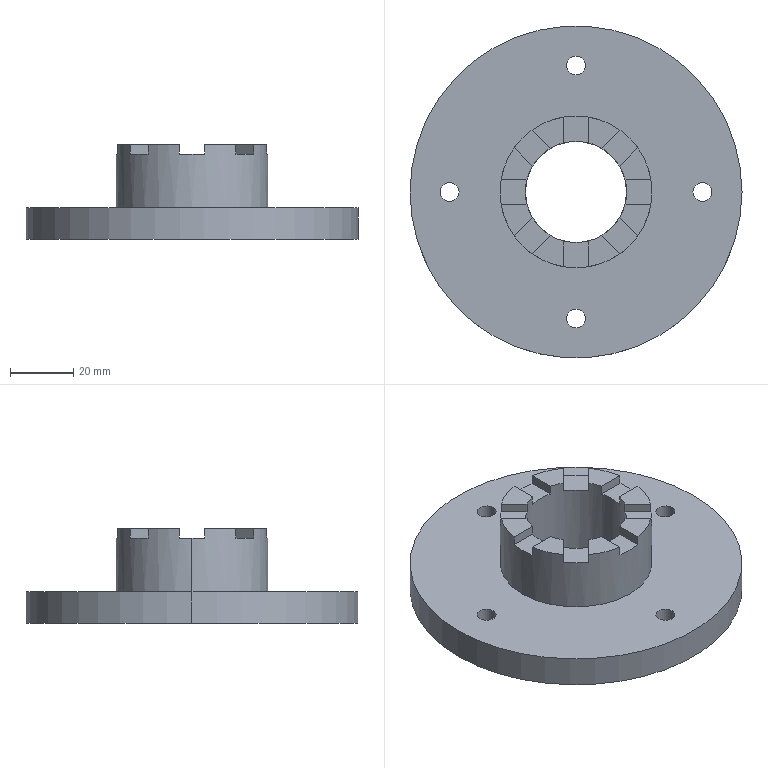Part | SolidWorks | features ICE 2, Extrusion 1 | 1 solid | 48 faces | box 105 x 105 x 30 mm | volume 95976 mm3 | plane 34 | cylinder 14 | commonest cylinder face diameters 6 x8 32 x2 48 x2 105 x2
STEP:
#1=CARTESIAN_POINT('',(24.,0.,27.));
#2=VERTEX_POINT('',#1);
#3=CARTESIAN_POINT('',(23.664,4.,27.));
#4=VERTEX_POINT('',#3);
#5=CARTESIAN_POINT('',(0.,0.,27.));
#6=DIRECTION('',(0.,0.,1.));
#7=DIRECTION('',(1.,0.,0.));
#8=AXIS2_PLACEMENT_3D('',#5,#6,#7);
#9=CIRCLE('',#8,24.);
#10=EDGE_CURVE('',#2,#4,#9,.T.);
#11=ORIENTED_EDGE('',*,*,#10,.F.);
#12=CARTESIAN_POINT('',(24.,0.,10.));
#13=VERTEX_POINT('',#12);
#14=CARTESIAN_POINT('',(24.,0.,30.));
#15=DIRECTION('',(0.,0.,-1.));
#16=VECTOR('',#15,1000.);
#17=LINE('',#14,#16);
#18=EDGE_CURVE('',#2,#13,#17,.T.);
#19=ORIENTED_EDGE('',*,*,#18,.T.);
#20=CARTESIAN_POINT('',(-24.,0.,10.));
#21=VERTEX_POINT('',#20);
#22=CARTESIAN_POINT('',(0.,0.,10.));
#23=DIRECTION('',(0.,0.,1.));
#24=DIRECTION('',(1.,0.,0.));
#25=AXIS2_PLACEMENT_3D('',#22,#23,#24);
#26=CIRCLE('',#25,24.);
#27=EDGE_CURVE('',#13,#21,#26,.T.);
#28=ORIENTED_EDGE('',*,*,#27,.T.);
#29=CARTESIAN_POINT('',(-24.,0.,27.));
#30=VERTEX_POINT('',#29);
#31=CARTESIAN_POINT('',(-24.,0.,30.));
#32=DIRECTION('',(0.,0.,-1.));
#33=VECTOR('',#32,1000.);
#34=LINE('',#31,#33);
#35=EDGE_CURVE('',#30,#21,#34,.T.);
#36=ORIENTED_EDGE('',*,*,#35,.F.);
#37=CARTESIAN_POINT('',(-23.664,4.,27.));
#38=VERTEX_POINT('',#37);
#39=CARTESIAN_POINT('',(0.,0.,27.));
#40=DIRECTION('',(0.,0.,1.));
#41=DIRECTION('',(1.,0.,0.));
#42=AXIS2_PLACEMENT_3D('',#39,#40,#41);
#43=CIRCLE('',#42,24.);
#44=EDGE_CURVE('',#38,#30,#43,.T.);
#45=ORIENTED_EDGE('',*,*,#44,.F.);
#46=CARTESIAN_POINT('',(-23.664,4.,30.));
#47=VERTEX_POINT('',#46);
#48=CARTESIAN_POINT('',(-23.664,4.,27.));
#49=DIRECTION('',(0.,0.,1.));
#50=VECTOR('',#49,1000.);
#51=LINE('',#48,#50);
#52=EDGE_CURVE('',#38,#47,#51,.T.);
#53=ORIENTED_EDGE('',*,*,#52,.T.);
#54=CARTESIAN_POINT('',(-19.562,13.905,30.));
#55=VERTEX_POINT('',#54);
#56=CARTESIAN_POINT('',(0.,0.,30.));
#57=DIRECTION('',(0.,0.,1.));
#58=DIRECTION('',(1.,0.,0.));
#59=AXIS2_PLACEMENT_3D('',#56,#57,#58);
#60=CIRCLE('',#59,24.);
#61=EDGE_CURVE('',#55,#47,#60,.T.);
#62=ORIENTED_EDGE('',*,*,#61,.F.);
#63=CARTESIAN_POINT('',(-19.562,13.905,27.));
#64=VERTEX_POINT('',#63);
#65=CARTESIAN_POINT('',(-19.562,13.905,27.));
#66=DIRECTION('',(0.,0.,1.));
#67=VECTOR('',#66,1000.);
#68=LINE('',#65,#67);
#69=EDGE_CURVE('',#64,#55,#68,.T.);
#70=ORIENTED_EDGE('',*,*,#69,.F.);
#71=CARTESIAN_POINT('',(-13.905,19.562,27.));
#72=VERTEX_POINT('',#71);
#73=CARTESIAN_POINT('',(0.,0.,27.));
#74=DIRECTION('',(0.,0.,1.));
#75=DIRECTION('',(1.,0.,0.));
#76=AXIS2_PLACEMENT_3D('',#73,#74,#75);
#77=CIRCLE('',#76,24.);
#78=EDGE_CURVE('',#72,#64,#77,.T.);
#79=ORIENTED_EDGE('',*,*,#78,.F.);
#80=CARTESIAN_POINT('',(-13.905,19.562,30.));
#81=VERTEX_POINT('',#80);
#82=CARTESIAN_POINT('',(-13.905,19.562,27.));
#83=DIRECTION('',(0.,0.,1.));
#84=VECTOR('',#83,1000.);
#85=LINE('',#82,#84);
#86=EDGE_CURVE('',#72,#81,#85,.T.);
#87=ORIENTED_EDGE('',*,*,#86,.T.);
#88=CARTESIAN_POINT('',(-4.,23.664,30.));
#89=VERTEX_POINT('',#88);
#90=CARTESIAN_POINT('',(0.,0.,30.));
#91=DIRECTION('',(0.,0.,1.));
#92=DIRECTION('',(1.,0.,0.));
#93=AXIS2_PLACEMENT_3D('',#90,#91,#92);
#94=CIRCLE('',#93,24.);
#95=EDGE_CURVE('',#89,#81,#94,.T.);
#96=ORIENTED_EDGE('',*,*,#95,.F.);
#97=CARTESIAN_POINT('',(-4.,23.664,27.));
#98=VERTEX_POINT('',#97);
#99=CARTESIAN_POINT('',(-4.,23.664,27.));
#100=DIRECTION('',(0.,0.,1.));
#101=VECTOR('',#100,1000.);
#102=LINE('',#99,#101);
#103=EDGE_CURVE('',#98,#89,#102,.T.);
#104=ORIENTED_EDGE('',*,*,#103,.F.);
#105=CARTESIAN_POINT('',(4.,23.664,27.));
#106=VERTEX_POINT('',#105);
#107=CARTESIAN_POINT('',(0.,0.,27.));
#108=DIRECTION('',(0.,0.,1.));
#109=DIRECTION('',(1.,0.,0.));
#110=AXIS2_PLACEMENT_3D('',#107,#108,#109);
#111=CIRCLE('',#110,24.);
#112=EDGE_CURVE('',#106,#98,#111,.T.);
#113=ORIENTED_EDGE('',*,*,#112,.F.);
#114=CARTESIAN_POINT('',(4.,23.664,30.));
#115=VERTEX_POINT('',#114);
#116=CARTESIAN_POINT('',(4.,23.664,27.));
#117=DIRECTION('',(0.,0.,1.));
#118=VECTOR('',#117,1000.);
#119=LINE('',#116,#118);
#120=EDGE_CURVE('',#106,#115,#119,.T.);
#121=ORIENTED_EDGE('',*,*,#120,.T.);
#122=CARTESIAN_POINT('',(13.905,19.562,30.));
#123=VERTEX_POINT('',#122);
#124=CARTESIAN_POINT('',(0.,0.,30.));
#125=DIRECTION('',(0.,0.,1.));
#126=DIRECTION('',(1.,0.,0.));
#127=AXIS2_PLACEMENT_3D('',#124,#125,#126);
#128=CIRCLE('',#127,24.);
#129=EDGE_CURVE('',#123,#115,#128,.T.);
#130=ORIENTED_EDGE('',*,*,#129,.F.);
#131=CARTESIAN_POINT('',(13.905,19.562,27.));
#132=VERTEX_POINT('',#131);
#133=CARTESIAN_POINT('',(13.905,19.562,27.));
#134=DIRECTION('',(0.,0.,1.));
#135=VECTOR('',#134,1000.);
#136=LINE('',#133,#135);
#137=EDGE_CURVE('',#132,#123,#136,.T.);
#138=ORIENTED_EDGE('',*,*,#137,.F.);
#139=CARTESIAN_POINT('',(19.562,13.905,27.));
#140=VERTEX_POINT('',#139);
#141=CARTESIAN_POINT('',(0.,0.,27.));
#142=DIRECTION('',(0.,0.,1.));
#143=DIRECTION('',(1.,0.,0.));
#144=AXIS2_PLACEMENT_3D('',#141,#142,#143);
#145=CIRCLE('',#144,24.);
#146=EDGE_CURVE('',#140,#132,#145,.T.);
#147=ORIENTED_EDGE('',*,*,#146,.F.);
#148=CARTESIAN_POINT('',(19.562,13.905,30.));
#149=VERTEX_POINT('',#148);
#150=CARTESIAN_POINT('',(19.562,13.905,27.));
#151=DIRECTION('',(0.,0.,1.));
#152=VECTOR('',#151,1000.);
#153=LINE('',#150,#152);
#154=EDGE_CURVE('',#140,#149,#153,.T.);
#155=ORIENTED_EDGE('',*,*,#154,.T.);
#156=CARTESIAN_POINT('',(23.664,4.,30.));
#157=VERTEX_POINT('',#156);
#158=CARTESIAN_POINT('',(0.,0.,30.));
#159=DIRECTION('',(0.,0.,1.));
#160=DIRECTION('',(1.,0.,0.));
#161=AXIS2_PLACEMENT_3D('',#158,#159,#160);
#162=CIRCLE('',#161,24.);
#163=EDGE_CURVE('',#157,#149,#162,.T.);
#164=ORIENTED_EDGE('',*,*,#163,.F.);
#165=CARTESIAN_POINT('',(23.664,4.,27.));
#166=DIRECTION('',(0.,0.,1.));
#167=VECTOR('',#166,1000.);
#168=LINE('',#165,#167);
#169=EDGE_CURVE('',#4,#157,#168,.T.);
#170=ORIENTED_EDGE('',*,*,#169,.F.);
#171=EDGE_LOOP('',(#11,#19,#28,#36,#45,#53,#62,#70,#79,#87,#96,#104,#113,#121,#130,#138,#147,#155,#164,#170));
#172=FACE_OUTER_BOUND('',#171,.T.);
#173=CARTESIAN_POINT('',(0.,0.,30.));
#174=DIRECTION('',(0.,0.,-1.));
#175=DIRECTION('',(-1.,0.,0.));
#176=AXIS2_PLACEMENT_3D('',#173,#174,#175);
#177=CYLINDRICAL_SURFACE('',#176,24.);
#178=ADVANCED_FACE('',(#172),#177,.T.);
#179=CARTESIAN_POINT('',(16.,0.,27.));
#180=VERTEX_POINT('',#179);
#181=CARTESIAN_POINT('',(15.492,-4.,27.));
#182=VERTEX_POINT('',#181);
#183=CARTESIAN_POINT('',(0.,0.,27.));
#184=DIRECTION('',(0.,0.,-1.));
#185=DIRECTION('',(1.,0.,0.));
#186=AXIS2_PLACEMENT_3D('',#183,#184,#185);
#187=CIRCLE('',#186,16.);
#188=EDGE_CURVE('',#180,#182,#187,.T.);
#189=ORIENTED_EDGE('',*,*,#188,.F.);
#190=CARTESIAN_POINT('',(16.,0.,0.));
#191=VERTEX_POINT('',#190);
#192=CARTESIAN_POINT('',(16.,0.,10.));
#193=DIRECTION('',(0.,0.,-1.));
#194=VECTOR('',#193,1000.);
#195=LINE('',#192,#194);
#196=EDGE_CURVE('',#180,#191,#195,.T.);
#197=ORIENTED_EDGE('',*,*,#196,.T.);
#198=CARTESIAN_POINT('',(-16.,0.,0.));
#199=VERTEX_POINT('',#198);
#200=CARTESIAN_POINT('',(0.,0.,0.));
#201=DIRECTION('',(0.,0.,1.));
#202=DIRECTION('',(1.,0.,0.));
#203=AXIS2_PLACEMENT_3D('',#200,#201,#202);
#204=CIRCLE('',#203,16.);
#205=EDGE_CURVE('',#199,#191,#204,.T.);
#206=ORIENTED_EDGE('',*,*,#205,.F.);
#207=CARTESIAN_POINT('',(-16.,0.,27.));
#208=VERTEX_POINT('',#207);
#209=CARTESIAN_POINT('',(-16.,0.,10.));
#210=DIRECTION('',(0.,0.,-1.));
#211=VECTOR('',#210,1000.);
#212=LINE('',#209,#211);
#213=EDGE_CURVE('',#208,#199,#212,.T.);
#214=ORIENTED_EDGE('',*,*,#213,.F.);
#215=CARTESIAN_POINT('',(-15.492,-4.,27.));
#216=VERTEX_POINT('',#215);
#217=CARTESIAN_POINT('',(0.,0.,27.));
#218=DIRECTION('',(0.,0.,-1.));
#219=DIRECTION('',(1.,0.,0.));
#220=AXIS2_PLACEMENT_3D('',#217,#218,#219);
#221=CIRCLE('',#220,16.);
#222=EDGE_CURVE('',#216,#208,#221,.T.);
#223=ORIENTED_EDGE('',*,*,#222,.F.);
#224=CARTESIAN_POINT('',(-15.492,-4.,30.));
#225=VERTEX_POINT('',#224);
#226=CARTESIAN_POINT('',(-15.492,-4.,27.));
#227=DIRECTION('',(0.,0.,1.));
#228=VECTOR('',#227,1000.);
#229=LINE('',#226,#228);
#230=EDGE_CURVE('',#216,#225,#229,.T.);
#231=ORIENTED_EDGE('',*,*,#230,.T.);
#232=CARTESIAN_POINT('',(-13.783,-8.126,30.));
#233=VERTEX_POINT('',#232);
#234=CARTESIAN_POINT('',(0.,0.,30.));
#235=DIRECTION('',(0.,0.,1.));
#236=DIRECTION('',(1.,0.,0.));
#237=AXIS2_PLACEMENT_3D('',#234,#235,#236);
#238=CIRCLE('',#237,16.);
#239=EDGE_CURVE('',#225,#233,#238,.T.);
#240=ORIENTED_EDGE('',*,*,#239,.T.);
#241=CARTESIAN_POINT('',(-13.783,-8.126,27.));
#242=VERTEX_POINT('',#241);
#243=CARTESIAN_POINT('',(-13.783,-8.126,27.));
#244=DIRECTION('',(0.,0.,1.));
#245=VECTOR('',#244,1000.);
#246=LINE('',#243,#245);
#247=EDGE_CURVE('',#242,#233,#246,.T.);
#248=ORIENTED_EDGE('',*,*,#247,.F.);
#249=CARTESIAN_POINT('',(-8.126,-13.783,27.));
#250=VERTEX_POINT('',#249);
#251=CARTESIAN_POINT('',(0.,0.,27.));
#252=DIRECTION('',(0.,0.,-1.));
#253=DIRECTION('',(1.,0.,0.));
#254=AXIS2_PLACEMENT_3D('',#251,#252,#253);
#255=CIRCLE('',#254,16.);
#256=EDGE_CURVE('',#250,#242,#255,.T.);
#257=ORIENTED_EDGE('',*,*,#256,.F.);
#258=CARTESIAN_POINT('',(-8.126,-13.783,30.));
#259=VERTEX_POINT('',#258);
#260=CARTESIAN_POINT('',(-8.126,-13.783,27.));
#261=DIRECTION('',(0.,0.,1.));
#262=VECTOR('',#261,1000.);
#263=LINE('',#260,#262);
#264=EDGE_CURVE('',#250,#259,#263,.T.);
#265=ORIENTED_EDGE('',*,*,#264,.T.);
#266=CARTESIAN_POINT('',(-4.,-15.492,30.));
#267=VERTEX_POINT('',#266);
#268=CARTESIAN_POINT('',(0.,0.,30.));
#269=DIRECTION('',(0.,0.,1.));
#270=DIRECTION('',(1.,0.,0.));
#271=AXIS2_PLACEMENT_3D('',#268,#269,#270);
#272=CIRCLE('',#271,16.);
#273=EDGE_CURVE('',#259,#267,#272,.T.);
#274=ORIENTED_EDGE('',*,*,#273,.T.);
#275=CARTESIAN_POINT('',(-4.,-15.492,27.));
#276=VERTEX_POINT('',#275);
#277=CARTESIAN_POINT('',(-4.,-15.492,27.));
#278=DIRECTION('',(0.,0.,1.));
#279=VECTOR('',#278,1000.);
#280=LINE('',#277,#279);
#281=EDGE_CURVE('',#276,#267,#280,.T.);
#282=ORIENTED_EDGE('',*,*,#281,.F.);
#283=CARTESIAN_POINT('',(4.,-15.492,27.));
#284=VERTEX_POINT('',#283);
#285=CARTESIAN_POINT('',(0.,0.,27.));
#286=DIRECTION('',(0.,0.,-1.));
#287=DIRECTION('',(1.,0.,0.));
#288=AXIS2_PLACEMENT_3D('',#285,#286,#287);
#289=CIRCLE('',#288,16.);
#290=EDGE_CURVE('',#284,#276,#289,.T.);
#291=ORIENTED_EDGE('',*,*,#290,.F.);
#292=CARTESIAN_POINT('',(4.,-15.492,30.));
#293=VERTEX_POINT('',#292);
#294=CARTESIAN_POINT('',(4.,-15.492,27.));
#295=DIRECTION('',(0.,0.,1.));
#296=VECTOR('',#295,1000.);
#297=LINE('',#294,#296);
#298=EDGE_CURVE('',#284,#293,#297,.T.);
#299=ORIENTED_EDGE('',*,*,#298,.T.);
#300=CARTESIAN_POINT('',(8.126,-13.783,30.));
#301=VERTEX_POINT('',#300);
#302=CARTESIAN_POINT('',(0.,0.,30.));
#303=DIRECTION('',(0.,0.,1.));
#304=DIRECTION('',(1.,0.,0.));
#305=AXIS2_PLACEMENT_3D('',#302,#303,#304);
#306=CIRCLE('',#305,16.);
#307=EDGE_CURVE('',#293,#301,#306,.T.);
#308=ORIENTED_EDGE('',*,*,#307,.T.);
#309=CARTESIAN_POINT('',(8.126,-13.783,27.));
#310=VERTEX_POINT('',#309);
#311=CARTESIAN_POINT('',(8.126,-13.783,27.));
#312=DIRECTION('',(0.,0.,1.));
#313=VECTOR('',#312,1000.);
#314=LINE('',#311,#313);
#315=EDGE_CURVE('',#310,#301,#314,.T.);
#316=ORIENTED_EDGE('',*,*,#315,.F.);
#317=CARTESIAN_POINT('',(13.783,-8.126,27.));
#318=VERTEX_POINT('',#317);
#319=CARTESIAN_POINT('',(0.,0.,27.));
#320=DIRECTION('',(0.,0.,-1.));
#321=DIRECTION('',(1.,0.,0.));
#322=AXIS2_PLACEMENT_3D('',#319,#320,#321);
#323=CIRCLE('',#322,16.);
#324=EDGE_CURVE('',#318,#310,#323,.T.);
#325=ORIENTED_EDGE('',*,*,#324,.F.);
#326=CARTESIAN_POINT('',(13.783,-8.126,30.));
#327=VERTEX_POINT('',#326);
#328=CARTESIAN_POINT('',(13.783,-8.126,27.));
#329=DIRECTION('',(0.,0.,1.));
#330=VECTOR('',#329,1000.);
#331=LINE('',#328,#330);
#332=EDGE_CURVE('',#318,#327,#331,.T.);
#333=ORIENTED_EDGE('',*,*,#332,.T.);
#334=CARTESIAN_POINT('',(15.492,-4.,30.));
#335=VERTEX_POINT('',#334);
#336=CARTESIAN_POINT('',(0.,0.,30.));
#337=DIRECTION('',(0.,0.,1.));
#338=DIRECTION('',(1.,0.,0.));
#339=AXIS2_PLACEMENT_3D('',#336,#337,#338);
#340=CIRCLE('',#339,16.);
#341=EDGE_CURVE('',#327,#335,#340,.T.);
#342=ORIENTED_EDGE('',*,*,#341,.T.);
#343=CARTESIAN_POINT('',(15.492,-4.,27.));
#344=DIRECTION('',(0.,0.,1.));
#345=VECTOR('',#344,1000.);
#346=LINE('',#343,#345);
#347=EDGE_CURVE('',#182,#335,#346,.T.);
#348=ORIENTED_EDGE('',*,*,#347,.F.);
#349=EDGE_LOOP('',(#189,#197,#206,#214,#223,#231,#240,#248,#257,#265,#274,#282,#291,#299,#308,#316,#325,#333,#342,#348));
#350=FACE_OUTER_BOUND('',#349,.T.);
#351=CARTESIAN_POINT('',(0.,0.,10.));
#352=DIRECTION('',(0.,0.,-1.));
#353=DIRECTION('',(-1.,0.,0.));
#354=AXIS2_PLACEMENT_3D('',#351,#352,#353);
#355=CYLINDRICAL_SURFACE('',#354,16.);
#356=ADVANCED_FACE('',(#350),#355,.F.);
#357=CARTESIAN_POINT('',(-43.,0.,10.));
#358=VERTEX_POINT('',#357);
#359=CARTESIAN_POINT('',(-37.,0.,10.));
#360=VERTEX_POINT('',#359);
#361=CARTESIAN_POINT('',(-40.,0.,10.));
#362=DIRECTION('',(0.,0.,1.));
#363=DIRECTION('',(1.,0.,0.));
#364=AXIS2_PLACEMENT_3D('',#361,#362,#363);
#365=CIRCLE('',#364,3.);
#366=EDGE_CURVE('',#358,#360,#365,.T.);
#367=ORIENTED_EDGE('',*,*,#366,.T.);
#368=CARTESIAN_POINT('',(-37.,0.,0.));
#369=VERTEX_POINT('',#368);
#370=CARTESIAN_POINT('',(-37.,0.,10.));
#371=DIRECTION('',(0.,0.,-1.));
#372=VECTOR('',#371,1000.);
#373=LINE('',#370,#372);
#374=EDGE_CURVE('',#360,#369,#373,.T.);
#375=ORIENTED_EDGE('',*,*,#374,.T.);
#376=CARTESIAN_POINT('',(-43.,0.,0.));
#377=VERTEX_POINT('',#376);
#378=CARTESIAN_POINT('',(-40.,0.,0.));
#379=DIRECTION('',(0.,0.,1.));
#380=DIRECTION('',(1.,0.,0.));
#381=AXIS2_PLACEMENT_3D('',#378,#379,#380);
#382=CIRCLE('',#381,3.);
#383=EDGE_CURVE('',#377,#369,#382,.T.);
#384=ORIENTED_EDGE('',*,*,#383,.F.);
#385=CARTESIAN_POINT('',(-43.,0.,10.));
#386=DIRECTION('',(0.,0.,-1.));
#387=VECTOR('',#386,1000.);
#388=LINE('',#385,#387);
#389=EDGE_CURVE('',#358,#377,#388,.T.);
#390=ORIENTED_EDGE('',*,*,#389,.F.);
#391=EDGE_LOOP('',(#367,#375,#384,#390));
#392=FACE_OUTER_BOUND('',#391,.T.);
#393=CARTESIAN_POINT('',(-40.,0.,10.));
#394=DIRECTION('',(0.,0.,-1.));
#395=DIRECTION('',(-1.,0.,0.));
#396=AXIS2_PLACEMENT_3D('',#393,#394,#395);
#397=CYLINDRICAL_SURFACE('',#396,3.);
#398=ADVANCED_FACE('',(#392),#397,.F.);
#399=CARTESIAN_POINT('',(-3.,-40.,10.));
#400=VERTEX_POINT('',#399);
#401=CARTESIAN_POINT('',(3.,-40.,10.));
#402=VERTEX_POINT('',#401);
#403=CARTESIAN_POINT('',(0.,-40.,10.));
#404=DIRECTION('',(0.,0.,1.));
#405=DIRECTION('',(1.,0.,0.));
#406=AXIS2_PLACEMENT_3D('',#403,#404,#405);
#407=CIRCLE('',#406,3.);
#408=EDGE_CURVE('',#400,#402,#407,.T.);
#409=ORIENTED_EDGE('',*,*,#408,.T.);
#410=CARTESIAN_POINT('',(3.,-40.,0.));
#411=VERTEX_POINT('',#410);
#412=CARTESIAN_POINT('',(3.,-40.,10.));
#413=DIRECTION('',(0.,0.,-1.));
#414=VECTOR('',#413,1000.);
#415=LINE('',#412,#414);
#416=EDGE_CURVE('',#402,#411,#415,.T.);
#417=ORIENTED_EDGE('',*,*,#416,.T.);
#418=CARTESIAN_POINT('',(-3.,-40.,0.));
#419=VERTEX_POINT('',#418);
#420=CARTESIAN_POINT('',(0.,-40.,0.));
#421=DIRECTION('',(0.,0.,1.));
#422=DIRECTION('',(1.,0.,0.));
#423=AXIS2_PLACEMENT_3D('',#420,#421,#422);
#424=CIRCLE('',#423,3.);
#425=EDGE_CURVE('',#419,#411,#424,.T.);
#426=ORIENTED_EDGE('',*,*,#425,.F.);
#427=CARTESIAN_POINT('',(-3.,-40.,10.));
#428=DIRECTION('',(0.,0.,-1.));
#429=VECTOR('',#428,1000.);
#430=LINE('',#427,#429);
#431=EDGE_CURVE('',#400,#419,#430,.T.);
#432=ORIENTED_EDGE('',*,*,#431,.F.);
#433=EDGE_LOOP('',(#409,#417,#426,#432));
#434=FACE_OUTER_BOUND('',#433,.T.);
#435=CARTESIAN_POINT('',(0.,-40.,10.));
#436=DIRECTION('',(0.,0.,-1.));
#437=DIRECTION('',(-1.,0.,0.));
#438=AXIS2_PLACEMENT_3D('',#435,#436,#437);
#439=CYLINDRICAL_SURFACE('',#438,3.);
#440=ADVANCED_FACE('',(#434),#439,.F.);
#441=CARTESIAN_POINT('',(37.,0.,10.));
#442=VERTEX_POINT('',#441);
#443=CARTESIAN_POINT('',(43.,0.,10.));
#444=VERTEX_POINT('',#443);
#445=CARTESIAN_POINT('',(40.,0.,10.));
#446=DIRECTION('',(0.,0.,1.));
#447=DIRECTION('',(1.,0.,0.));
#448=AXIS2_PLACEMENT_3D('',#445,#446,#447);
#449=CIRCLE('',#448,3.);
#450=EDGE_CURVE('',#442,#444,#449,.T.);
#451=ORIENTED_EDGE('',*,*,#450,.T.);
#452=CARTESIAN_POINT('',(43.,0.,0.));
#453=VERTEX_POINT('',#452);
#454=CARTESIAN_POINT('',(43.,0.,10.));
#455=DIRECTION('',(0.,0.,-1.));
#456=VECTOR('',#455,1000.);
#457=LINE('',#454,#456);
#458=EDGE_CURVE('',#444,#453,#457,.T.);
#459=ORIENTED_EDGE('',*,*,#458,.T.);
#460=CARTESIAN_POINT('',(37.,0.,0.));
#461=VERTEX_POINT('',#460);
#462=CARTESIAN_POINT('',(40.,0.,0.));
#463=DIRECTION('',(0.,0.,1.));
#464=DIRECTION('',(1.,0.,0.));
#465=AXIS2_PLACEMENT_3D('',#462,#463,#464);
#466=CIRCLE('',#465,3.);
#467=EDGE_CURVE('',#461,#453,#466,.T.);
#468=ORIENTED_EDGE('',*,*,#467,.F.);
#469=CARTESIAN_POINT('',(37.,0.,10.));
#470=DIRECTION('',(0.,0.,-1.));
#471=VECTOR('',#470,1000.);
#472=LINE('',#469,#471);
#473=EDGE_CURVE('',#442,#461,#472,.T.);
#474=ORIENTED_EDGE('',*,*,#473,.F.);
#475=EDGE_LOOP('',(#451,#459,#468,#474));
#476=FACE_OUTER_BOUND('',#475,.T.);
#477=CARTESIAN_POINT('',(40.,0.,10.));
#478=DIRECTION('',(0.,0.,-1.));
#479=DIRECTION('',(-1.,0.,0.));
#480=AXIS2_PLACEMENT_3D('',#477,#478,#479);
#481=CYLINDRICAL_SURFACE('',#480,3.);
#482=ADVANCED_FACE('',(#476),#481,.F.);
#483=CARTESIAN_POINT('',(-3.,40.,10.));
#484=VERTEX_POINT('',#483);
#485=CARTESIAN_POINT('',(3.,40.,10.));
#486=VERTEX_POINT('',#485);
#487=CARTESIAN_POINT('',(0.,40.,10.));
#488=DIRECTION('',(0.,0.,1.));
#489=DIRECTION('',(1.,0.,0.));
#490=AXIS2_PLACEMENT_3D('',#487,#488,#489);
#491=CIRCLE('',#490,3.);
#492=EDGE_CURVE('',#484,#486,#491,.T.);
#493=ORIENTED_EDGE('',*,*,#492,.T.);
#494=CARTESIAN_POINT('',(3.,40.,0.));
#495=VERTEX_POINT('',#494);
#496=CARTESIAN_POINT('',(3.,40.,10.));
#497=DIRECTION('',(0.,0.,-1.));
#498=VECTOR('',#497,1000.);
#499=LINE('',#496,#498);
#500=EDGE_CURVE('',#486,#495,#499,.T.);
#501=ORIENTED_EDGE('',*,*,#500,.T.);
#502=CARTESIAN_POINT('',(-3.,40.,0.));
#503=VERTEX_POINT('',#502);
#504=CARTESIAN_POINT('',(0.,40.,0.));
#505=DIRECTION('',(0.,0.,1.));
#506=DIRECTION('',(1.,0.,0.));
#507=AXIS2_PLACEMENT_3D('',#504,#505,#506);
#508=CIRCLE('',#507,3.);
#509=EDGE_CURVE('',#503,#495,#508,.T.);
#510=ORIENTED_EDGE('',*,*,#509,.F.);
#511=CARTESIAN_POINT('',(-3.,40.,10.));
#512=DIRECTION('',(0.,0.,-1.));
#513=VECTOR('',#512,1000.);
#514=LINE('',#511,#513);
#515=EDGE_CURVE('',#484,#503,#514,.T.);
#516=ORIENTED_EDGE('',*,*,#515,.F.);
#517=EDGE_LOOP('',(#493,#501,#510,#516));
#518=FACE_OUTER_BOUND('',#517,.T.);
#519=CARTESIAN_POINT('',(0.,40.,10.));
#520=DIRECTION('',(0.,0.,-1.));
#521=DIRECTION('',(-1.,0.,0.));
#522=AXIS2_PLACEMENT_3D('',#519,#520,#521);
#523=CYLINDRICAL_SURFACE('',#522,3.);
#524=ADVANCED_FACE('',(#518),#523,.F.);
#525=CARTESIAN_POINT('',(52.5,0.,10.));
#526=VERTEX_POINT('',#525);
#527=CARTESIAN_POINT('',(-52.5,0.,10.));
#528=VERTEX_POINT('',#527);
#529=CARTESIAN_POINT('',(0.,0.,10.));
#530=DIRECTION('',(0.,0.,1.));
#531=DIRECTION('',(1.,0.,0.));
#532=AXIS2_PLACEMENT_3D('',#529,#530,#531);
#533=CIRCLE('',#532,52.5);
#534=EDGE_CURVE('',#526,#528,#533,.T.);
#535=ORIENTED_EDGE('',*,*,#534,.F.);
#536=CARTESIAN_POINT('',(52.5,0.,0.));
#537=VERTEX_POINT('',#536);
#538=CARTESIAN_POINT('',(52.5,0.,10.));
#539=DIRECTION('',(0.,0.,-1.));
#540=VECTOR('',#539,1000.);
#541=LINE('',#538,#540);
#542=EDGE_CURVE('',#526,#537,#541,.T.);
#543=ORIENTED_EDGE('',*,*,#542,.T.);
#544=CARTESIAN_POINT('',(-52.5,0.,0.));
#545=VERTEX_POINT('',#544);
#546=CARTESIAN_POINT('',(0.,0.,0.));
#547=DIRECTION('',(0.,0.,1.));
#548=DIRECTION('',(1.,0.,0.));
#549=AXIS2_PLACEMENT_3D('',#546,#547,#548);
#550=CIRCLE('',#549,52.5);
#551=EDGE_CURVE('',#537,#545,#550,.T.);
#552=ORIENTED_EDGE('',*,*,#551,.T.);
#553=CARTESIAN_POINT('',(-52.5,0.,10.));
#554=DIRECTION('',(0.,0.,-1.));
#555=VECTOR('',#554,1000.);
#556=LINE('',#553,#555);
#557=EDGE_CURVE('',#528,#545,#556,.T.);
#558=ORIENTED_EDGE('',*,*,#557,.F.);
#559=EDGE_LOOP('',(#535,#543,#552,#558));
#560=FACE_OUTER_BOUND('',#559,.T.);
#561=CARTESIAN_POINT('',(0.,0.,10.));
#562=DIRECTION('',(0.,0.,-1.));
#563=DIRECTION('',(-1.,0.,0.));
#564=AXIS2_PLACEMENT_3D('',#561,#562,#563);
#565=CYLINDRICAL_SURFACE('',#564,52.5);
#566=ADVANCED_FACE('',(#560),#565,.T.);
#567=CARTESIAN_POINT('',(-8.126,13.783,30.));
#568=VERTEX_POINT('',#567);
#569=CARTESIAN_POINT('',(-13.905,19.562,30.));
#570=DIRECTION('',(-0.7071,0.7071,0.));
#571=VECTOR('',#570,1000.);
#572=LINE('',#569,#571);
#573=EDGE_CURVE('',#568,#81,#572,.T.);
#574=ORIENTED_EDGE('',*,*,#573,.F.);
#575=CARTESIAN_POINT('',(-4.,15.492,30.));
#576=VERTEX_POINT('',#575);
#577=CARTESIAN_POINT('',(0.,0.,30.));
#578=DIRECTION('',(0.,0.,1.));
#579=DIRECTION('',(1.,0.,0.));
#580=AXIS2_PLACEMENT_3D('',#577,#578,#579);
#581=CIRCLE('',#580,16.);
#582=EDGE_CURVE('',#576,#568,#581,.T.);
#583=ORIENTED_EDGE('',*,*,#582,.F.);
#584=CARTESIAN_POINT('',(-4.,23.664,30.));
#585=DIRECTION('',(0.,-1.,0.));
#586=VECTOR('',#585,1000.);
#587=LINE('',#584,#586);
#588=EDGE_CURVE('',#89,#576,#587,.T.);
#589=ORIENTED_EDGE('',*,*,#588,.F.);
#590=ORIENTED_EDGE('',*,*,#95,.T.);
#591=EDGE_LOOP('',(#574,#583,#589,#590));
#592=FACE_OUTER_BOUND('',#591,.T.);
#593=CARTESIAN_POINT('',(0.,0.,30.));
#594=DIRECTION('',(0.,0.,1.));
#595=DIRECTION('',(1.,0.,0.));
#596=AXIS2_PLACEMENT_3D('',#593,#594,#595);
#597=PLANE('',#596);
#598=ADVANCED_FACE('',(#592),#597,.T.);
#599=CARTESIAN_POINT('',(-13.783,8.126,30.));
#600=VERTEX_POINT('',#599);
#601=CARTESIAN_POINT('',(-19.562,13.905,30.));
#602=DIRECTION('',(0.7071,-0.7071,0.));
#603=VECTOR('',#602,1000.);
#604=LINE('',#601,#603);
#605=EDGE_CURVE('',#55,#600,#604,.T.);
#606=ORIENTED_EDGE('',*,*,#605,.F.);
#607=ORIENTED_EDGE('',*,*,#61,.T.);
#608=CARTESIAN_POINT('',(-15.492,4.,30.));
#609=VERTEX_POINT('',#608);
#610=CARTESIAN_POINT('',(-23.664,4.,30.));
#611=DIRECTION('',(-1.,0.,0.));
#612=VECTOR('',#611,1000.);
#613=LINE('',#610,#612);
#614=EDGE_CURVE('',#609,#47,#613,.T.);
#615=ORIENTED_EDGE('',*,*,#614,.F.);
#616=CARTESIAN_POINT('',(0.,0.,30.));
#617=DIRECTION('',(0.,0.,1.));
#618=DIRECTION('',(1.,0.,0.));
#619=AXIS2_PLACEMENT_3D('',#616,#617,#618);
#620=CIRCLE('',#619,16.);
#621=EDGE_CURVE('',#600,#609,#620,.T.);
#622=ORIENTED_EDGE('',*,*,#621,.F.);
#623=EDGE_LOOP('',(#606,#607,#615,#622));
#624=FACE_OUTER_BOUND('',#623,.T.);
#625=CARTESIAN_POINT('',(0.,0.,30.));
#626=DIRECTION('',(0.,0.,1.));
#627=DIRECTION('',(1.,0.,0.));
#628=AXIS2_PLACEMENT_3D('',#625,#626,#627);
#629=PLANE('',#628);
#630=ADVANCED_FACE('',(#624),#629,.T.);
#631=CARTESIAN_POINT('',(-23.664,-4.,30.));
#632=VERTEX_POINT('',#631);
#633=CARTESIAN_POINT('',(-23.664,-4.,30.));
#634=DIRECTION('',(1.,0.,0.));
#635=VECTOR('',#634,1000.);
#636=LINE('',#633,#635);
#637=EDGE_CURVE('',#632,#225,#636,.T.);
#638=ORIENTED_EDGE('',*,*,#637,.F.);
#639=CARTESIAN_POINT('',(-19.562,-13.905,30.));
#640=VERTEX_POINT('',#639);
#641=CARTESIAN_POINT('',(0.,0.,30.));
#642=DIRECTION('',(0.,0.,1.));
#643=DIRECTION('',(1.,0.,0.));
#644=AXIS2_PLACEMENT_3D('',#641,#642,#643);
#645=CIRCLE('',#644,24.);
#646=EDGE_CURVE('',#632,#640,#645,.T.);
#647=ORIENTED_EDGE('',*,*,#646,.T.);
#648=CARTESIAN_POINT('',(-19.562,-13.905,30.));
#649=DIRECTION('',(-0.7071,-0.7071,0.));
#650=VECTOR('',#649,1000.);
#651=LINE('',#648,#650);
#652=EDGE_CURVE('',#233,#640,#651,.T.);
#653=ORIENTED_EDGE('',*,*,#652,.F.);
#654=ORIENTED_EDGE('',*,*,#239,.F.);
#655=EDGE_LOOP('',(#638,#647,#653,#654));
#656=FACE_OUTER_BOUND('',#655,.T.);
#657=CARTESIAN_POINT('',(0.,0.,30.));
#658=DIRECTION('',(0.,0.,1.));
#659=DIRECTION('',(1.,0.,0.));
#660=AXIS2_PLACEMENT_3D('',#657,#658,#659);
#661=PLANE('',#660);
#662=ADVANCED_FACE('',(#656),#661,.T.);
#663=CARTESIAN_POINT('',(-13.905,-19.562,30.));
#664=VERTEX_POINT('',#663);
#665=CARTESIAN_POINT('',(-13.905,-19.562,30.));
#666=DIRECTION('',(0.7071,0.7071,0.));
#667=VECTOR('',#666,1000.);
#668=LINE('',#665,#667);
#669=EDGE_CURVE('',#664,#259,#668,.T.);
#670=ORIENTED_EDGE('',*,*,#669,.F.);
#671=CARTESIAN_POINT('',(-4.,-23.664,30.));
#672=VERTEX_POINT('',#671);
#673=CARTESIAN_POINT('',(0.,0.,30.));
#674=DIRECTION('',(0.,0.,1.));
#675=DIRECTION('',(1.,0.,0.));
#676=AXIS2_PLACEMENT_3D('',#673,#674,#675);
#677=CIRCLE('',#676,24.);
#678=EDGE_CURVE('',#664,#672,#677,.T.);
#679=ORIENTED_EDGE('',*,*,#678,.T.);
#680=CARTESIAN_POINT('',(-4.,-23.664,30.));
#681=DIRECTION('',(0.,-1.,0.));
#682=VECTOR('',#681,1000.);
#683=LINE('',#680,#682);
#684=EDGE_CURVE('',#267,#672,#683,.T.);
#685=ORIENTED_EDGE('',*,*,#684,.F.);
#686=ORIENTED_EDGE('',*,*,#273,.F.);
#687=EDGE_LOOP('',(#670,#679,#685,#686));
#688=FACE_OUTER_BOUND('',#687,.T.);
#689=CARTESIAN_POINT('',(0.,0.,30.));
#690=DIRECTION('',(0.,0.,1.));
#691=DIRECTION('',(1.,0.,0.));
#692=AXIS2_PLACEMENT_3D('',#689,#690,#691);
#693=PLANE('',#692);
#694=ADVANCED_FACE('',(#688),#693,.T.);
#695=CARTESIAN_POINT('',(4.,-23.664,30.));
#696=VERTEX_POINT('',#695);
#697=CARTESIAN_POINT('',(4.,-23.664,30.));
#698=DIRECTION('',(0.,1.,0.));
#699=VECTOR('',#698,1000.);
#700=LINE('',#697,#699);
#701=EDGE_CURVE('',#696,#293,#700,.T.);
#702=ORIENTED_EDGE('',*,*,#701,.F.);
#703=CARTESIAN_POINT('',(13.905,-19.562,30.));
#704=VERTEX_POINT('',#703);
#705=CARTESIAN_POINT('',(0.,0.,30.));
#706=DIRECTION('',(0.,0.,1.));
#707=DIRECTION('',(1.,0.,0.));
#708=AXIS2_PLACEMENT_3D('',#705,#706,#707);
#709=CIRCLE('',#708,24.);
#710=EDGE_CURVE('',#696,#704,#709,.T.);
#711=ORIENTED_EDGE('',*,*,#710,.T.);
#712=CARTESIAN_POINT('',(13.905,-19.562,30.));
#713=DIRECTION('',(0.7071,-0.7071,0.));
#714=VECTOR('',#713,1000.);
#715=LINE('',#712,#714);
#716=EDGE_CURVE('',#301,#704,#715,.T.);
#717=ORIENTED_EDGE('',*,*,#716,.F.);
#718=ORIENTED_EDGE('',*,*,#307,.F.);
#719=EDGE_LOOP('',(#702,#711,#717,#718));
#720=FACE_OUTER_BOUND('',#719,.T.);
#721=CARTESIAN_POINT('',(0.,0.,30.));
#722=DIRECTION('',(0.,0.,1.));
#723=DIRECTION('',(1.,0.,0.));
#724=AXIS2_PLACEMENT_3D('',#721,#722,#723);
#725=PLANE('',#724);
#726=ADVANCED_FACE('',(#720),#725,.T.);
#727=CARTESIAN_POINT('',(19.562,-13.905,30.));
#728=VERTEX_POINT('',#727);
#729=CARTESIAN_POINT('',(19.562,-13.905,30.));
#730=DIRECTION('',(-0.7071,0.7071,0.));
#731=VECTOR('',#730,1000.);
#732=LINE('',#729,#731);
#733=EDGE_CURVE('',#728,#327,#732,.T.);
#734=ORIENTED_EDGE('',*,*,#733,.F.);
#735=CARTESIAN_POINT('',(23.664,-4.,30.));
#736=VERTEX_POINT('',#735);
#737=CARTESIAN_POINT('',(0.,0.,30.));
#738=DIRECTION('',(0.,0.,1.));
#739=DIRECTION('',(1.,0.,0.));
#740=AXIS2_PLACEMENT_3D('',#737,#738,#739);
#741=CIRCLE('',#740,24.);
#742=EDGE_CURVE('',#728,#736,#741,.T.);
#743=ORIENTED_EDGE('',*,*,#742,.T.);
#744=CARTESIAN_POINT('',(23.664,-4.,30.));
#745=DIRECTION('',(1.,0.,0.));
#746=VECTOR('',#745,1000.);
#747=LINE('',#744,#746);
#748=EDGE_CURVE('',#335,#736,#747,.T.);
#749=ORIENTED_EDGE('',*,*,#748,.F.);
#750=ORIENTED_EDGE('',*,*,#341,.F.);
#751=EDGE_LOOP('',(#734,#743,#749,#750));
#752=FACE_OUTER_BOUND('',#751,.T.);
#753=CARTESIAN_POINT('',(0.,0.,30.));
#754=DIRECTION('',(0.,0.,1.));
#755=DIRECTION('',(1.,0.,0.));
#756=AXIS2_PLACEMENT_3D('',#753,#754,#755);
#757=PLANE('',#756);
#758=ADVANCED_FACE('',(#752),#757,.T.);
#759=CARTESIAN_POINT('',(15.492,4.,30.));
#760=VERTEX_POINT('',#759);
#761=CARTESIAN_POINT('',(23.664,4.,30.));
#762=DIRECTION('',(-1.,0.,0.));
#763=VECTOR('',#762,1000.);
#764=LINE('',#761,#763);
#765=EDGE_CURVE('',#157,#760,#764,.T.);
#766=ORIENTED_EDGE('',*,*,#765,.F.);
#767=ORIENTED_EDGE('',*,*,#163,.T.);
#768=CARTESIAN_POINT('',(13.783,8.126,30.));
#769=VERTEX_POINT('',#768);
#770=CARTESIAN_POINT('',(19.562,13.905,30.));
#771=DIRECTION('',(0.7071,0.7071,0.));
#772=VECTOR('',#771,1000.);
#773=LINE('',#770,#772);
#774=EDGE_CURVE('',#769,#149,#773,.T.);
#775=ORIENTED_EDGE('',*,*,#774,.F.);
#776=CARTESIAN_POINT('',(0.,0.,30.));
#777=DIRECTION('',(0.,0.,1.));
#778=DIRECTION('',(1.,0.,0.));
#779=AXIS2_PLACEMENT_3D('',#776,#777,#778);
#780=CIRCLE('',#779,16.);
#781=EDGE_CURVE('',#760,#769,#780,.T.);
#782=ORIENTED_EDGE('',*,*,#781,.F.);
#783=EDGE_LOOP('',(#766,#767,#775,#782));
#784=FACE_OUTER_BOUND('',#783,.T.);
#785=CARTESIAN_POINT('',(0.,0.,30.));
#786=DIRECTION('',(0.,0.,1.));
#787=DIRECTION('',(1.,0.,0.));
#788=AXIS2_PLACEMENT_3D('',#785,#786,#787);
#789=PLANE('',#788);
#790=ADVANCED_FACE('',(#784),#789,.T.);
#791=CARTESIAN_POINT('',(0.,0.,10.));
#792=DIRECTION('',(0.,0.,1.));
#793=DIRECTION('',(1.,0.,0.));
#794=AXIS2_PLACEMENT_3D('',#791,#792,#793);
#795=CIRCLE('',#794,52.5);
#796=EDGE_CURVE('',#528,#526,#795,.T.);
#797=ORIENTED_EDGE('',*,*,#796,.T.);
#798=ORIENTED_EDGE('',*,*,#534,.T.);
#799=EDGE_LOOP('',(#797,#798));
#800=FACE_OUTER_BOUND('',#799,.T.);
#801=ORIENTED_EDGE('',*,*,#492,.F.);
#802=CARTESIAN_POINT('',(0.,40.,10.));
#803=DIRECTION('',(0.,0.,1.));
#804=DIRECTION('',(1.,0.,0.));
#805=AXIS2_PLACEMENT_3D('',#802,#803,#804);
#806=CIRCLE('',#805,3.);
#807=EDGE_CURVE('',#486,#484,#806,.T.);
#808=ORIENTED_EDGE('',*,*,#807,.F.);
#809=EDGE_LOOP('',(#801,#808));
#810=FACE_BOUND('',#809,.T.);
#811=ORIENTED_EDGE('',*,*,#450,.F.);
#812=CARTESIAN_POINT('',(40.,0.,10.));
#813=DIRECTION('',(0.,0.,1.));
#814=DIRECTION('',(1.,0.,0.));
#815=AXIS2_PLACEMENT_3D('',#812,#813,#814);
#816=CIRCLE('',#815,3.);
#817=EDGE_CURVE('',#444,#442,#816,.T.);
#818=ORIENTED_EDGE('',*,*,#817,.F.);
#819=EDGE_LOOP('',(#811,#818));
#820=FACE_BOUND('',#819,.T.);
#821=ORIENTED_EDGE('',*,*,#408,.F.);
#822=CARTESIAN_POINT('',(0.,-40.,10.));
#823=DIRECTION('',(0.,0.,1.));
#824=DIRECTION('',(1.,0.,0.));
#825=AXIS2_PLACEMENT_3D('',#822,#823,#824);
#826=CIRCLE('',#825,3.);
#827=EDGE_CURVE('',#402,#400,#826,.T.);
#828=ORIENTED_EDGE('',*,*,#827,.F.);
#829=EDGE_LOOP('',(#821,#828));
#830=FACE_BOUND('',#829,.T.);
#831=ORIENTED_EDGE('',*,*,#366,.F.);
#832=CARTESIAN_POINT('',(-40.,0.,10.));
#833=DIRECTION('',(0.,0.,1.));
#834=DIRECTION('',(1.,0.,0.));
#835=AXIS2_PLACEMENT_3D('',#832,#833,#834);
#836=CIRCLE('',#835,3.);
#837=EDGE_CURVE('',#360,#358,#836,.T.);
#838=ORIENTED_EDGE('',*,*,#837,.F.);
#839=EDGE_LOOP('',(#831,#838));
#840=FACE_BOUND('',#839,.T.);
#841=CARTESIAN_POINT('',(0.,0.,10.));
#842=DIRECTION('',(0.,0.,1.));
#843=DIRECTION('',(1.,0.,0.));
#844=AXIS2_PLACEMENT_3D('',#841,#842,#843);
#845=CIRCLE('',#844,24.);
#846=EDGE_CURVE('',#21,#13,#845,.T.);
#847=ORIENTED_EDGE('',*,*,#846,.F.);
#848=ORIENTED_EDGE('',*,*,#27,.F.);
#849=EDGE_LOOP('',(#847,#848));
#850=FACE_BOUND('',#849,.T.);
#851=CARTESIAN_POINT('',(0.,0.,10.));
#852=DIRECTION('',(0.,0.,1.));
#853=DIRECTION('',(1.,0.,0.));
#854=AXIS2_PLACEMENT_3D('',#851,#852,#853);
#855=PLANE('',#854);
#856=ADVANCED_FACE('',(#800,#810,#820,#830,#840,#850),#855,.T.);
#857=ORIENTED_EDGE('',*,*,#542,.F.);
#858=ORIENTED_EDGE('',*,*,#796,.F.);
#859=ORIENTED_EDGE('',*,*,#557,.T.);
#860=CARTESIAN_POINT('',(0.,0.,0.));
#861=DIRECTION('',(0.,0.,1.));
#862=DIRECTION('',(1.,0.,0.));
#863=AXIS2_PLACEMENT_3D('',#860,#861,#862);
#864=CIRCLE('',#863,52.5);
#865=EDGE_CURVE('',#545,#537,#864,.T.);
#866=ORIENTED_EDGE('',*,*,#865,.T.);
#867=EDGE_LOOP('',(#857,#858,#859,#866));
#868=FACE_OUTER_BOUND('',#867,.T.);
#869=CARTESIAN_POINT('',(0.,0.,10.));
#870=DIRECTION('',(0.,0.,-1.));
#871=DIRECTION('',(-1.,0.,0.));
#872=AXIS2_PLACEMENT_3D('',#869,#870,#871);
#873=CYLINDRICAL_SURFACE('',#872,52.5);
#874=ADVANCED_FACE('',(#868),#873,.T.);
#875=ORIENTED_EDGE('',*,*,#500,.F.);
#876=ORIENTED_EDGE('',*,*,#807,.T.);
#877=ORIENTED_EDGE('',*,*,#515,.T.);
#878=CARTESIAN_POINT('',(0.,40.,0.));
#879=DIRECTION('',(0.,0.,1.));
#880=DIRECTION('',(1.,0.,0.));
#881=AXIS2_PLACEMENT_3D('',#878,#879,#880);
#882=CIRCLE('',#881,3.);
#883=EDGE_CURVE('',#495,#503,#882,.T.);
#884=ORIENTED_EDGE('',*,*,#883,.F.);
#885=EDGE_LOOP('',(#875,#876,#877,#884));
#886=FACE_OUTER_BOUND('',#885,.T.);
#887=CARTESIAN_POINT('',(0.,40.,10.));
#888=DIRECTION('',(0.,0.,-1.));
#889=DIRECTION('',(-1.,0.,0.));
#890=AXIS2_PLACEMENT_3D('',#887,#888,#889);
#891=CYLINDRICAL_SURFACE('',#890,3.);
#892=ADVANCED_FACE('',(#886),#891,.F.);
#893=ORIENTED_EDGE('',*,*,#458,.F.);
#894=ORIENTED_EDGE('',*,*,#817,.T.);
#895=ORIENTED_EDGE('',*,*,#473,.T.);
#896=CARTESIAN_POINT('',(40.,0.,0.));
#897=DIRECTION('',(0.,0.,1.));
#898=DIRECTION('',(1.,0.,0.));
#899=AXIS2_PLACEMENT_3D('',#896,#897,#898);
#900=CIRCLE('',#899,3.);
#901=EDGE_CURVE('',#453,#461,#900,.T.);
#902=ORIENTED_EDGE('',*,*,#901,.F.);
#903=EDGE_LOOP('',(#893,#894,#895,#902));
#904=FACE_OUTER_BOUND('',#903,.T.);
#905=CARTESIAN_POINT('',(40.,0.,10.));
#906=DIRECTION('',(0.,0.,-1.));
#907=DIRECTION('',(-1.,0.,0.));
#908=AXIS2_PLACEMENT_3D('',#905,#906,#907);
#909=CYLINDRICAL_SURFACE('',#908,3.);
#910=ADVANCED_FACE('',(#904),#909,.F.);
#911=ORIENTED_EDGE('',*,*,#416,.F.);
#912=ORIENTED_EDGE('',*,*,#827,.T.);
#913=ORIENTED_EDGE('',*,*,#431,.T.);
#914=CARTESIAN_POINT('',(0.,-40.,0.));
#915=DIRECTION('',(0.,0.,1.));
#916=DIRECTION('',(1.,0.,0.));
#917=AXIS2_PLACEMENT_3D('',#914,#915,#916);
#918=CIRCLE('',#917,3.);
#919=EDGE_CURVE('',#411,#419,#918,.T.);
#920=ORIENTED_EDGE('',*,*,#919,.F.);
#921=EDGE_LOOP('',(#911,#912,#913,#920));
#922=FACE_OUTER_BOUND('',#921,.T.);
#923=CARTESIAN_POINT('',(0.,-40.,10.));
#924=DIRECTION('',(0.,0.,-1.));
#925=DIRECTION('',(-1.,0.,0.));
#926=AXIS2_PLACEMENT_3D('',#923,#924,#925);
#927=CYLINDRICAL_SURFACE('',#926,3.);
#928=ADVANCED_FACE('',(#922),#927,.F.);
#929=ORIENTED_EDGE('',*,*,#374,.F.);
#930=ORIENTED_EDGE('',*,*,#837,.T.);
#931=ORIENTED_EDGE('',*,*,#389,.T.);
#932=CARTESIAN_POINT('',(-40.,0.,0.));
#933=DIRECTION('',(0.,0.,1.));
#934=DIRECTION('',(1.,0.,0.));
#935=AXIS2_PLACEMENT_3D('',#932,#933,#934);
#936=CIRCLE('',#935,3.);
#937=EDGE_CURVE('',#369,#377,#936,.T.);
#938=ORIENTED_EDGE('',*,*,#937,.F.);
#939=EDGE_LOOP('',(#929,#930,#931,#938));
#940=FACE_OUTER_BOUND('',#939,.T.);
#941=CARTESIAN_POINT('',(-40.,0.,10.));
#942=DIRECTION('',(0.,0.,-1.));
#943=DIRECTION('',(-1.,0.,0.));
#944=AXIS2_PLACEMENT_3D('',#941,#942,#943);
#945=CYLINDRICAL_SURFACE('',#944,3.);
#946=ADVANCED_FACE('',(#940),#945,.F.);
#947=ORIENTED_EDGE('',*,*,#196,.F.);
#948=CARTESIAN_POINT('',(15.492,4.,27.));
#949=VERTEX_POINT('',#948);
#950=CARTESIAN_POINT('',(0.,0.,27.));
#951=DIRECTION('',(0.,0.,-1.));
#952=DIRECTION('',(1.,0.,0.));
#953=AXIS2_PLACEMENT_3D('',#950,#951,#952);
#954=CIRCLE('',#953,16.);
#955=EDGE_CURVE('',#949,#180,#954,.T.);
#956=ORIENTED_EDGE('',*,*,#955,.F.);
#957=CARTESIAN_POINT('',(15.492,4.,27.));
#958=DIRECTION('',(0.,0.,1.));
#959=VECTOR('',#958,1000.);
#960=LINE('',#957,#959);
#961=EDGE_CURVE('',#949,#760,#960,.T.);
#962=ORIENTED_EDGE('',*,*,#961,.T.);
#963=ORIENTED_EDGE('',*,*,#781,.T.);
#964=CARTESIAN_POINT('',(13.783,8.126,27.));
#965=VERTEX_POINT('',#964);
#966=CARTESIAN_POINT('',(13.783,8.126,27.));
#967=DIRECTION('',(0.,0.,1.));
#968=VECTOR('',#967,1000.);
#969=LINE('',#966,#968);
#970=EDGE_CURVE('',#965,#769,#969,.T.);
#971=ORIENTED_EDGE('',*,*,#970,.F.);
#972=CARTESIAN_POINT('',(8.126,13.783,27.));
#973=VERTEX_POINT('',#972);
#974=CARTESIAN_POINT('',(0.,0.,27.));
#975=DIRECTION('',(0.,0.,-1.));
#976=DIRECTION('',(1.,0.,0.));
#977=AXIS2_PLACEMENT_3D('',#974,#975,#976);
#978=CIRCLE('',#977,16.);
#979=EDGE_CURVE('',#973,#965,#978,.T.);
#980=ORIENTED_EDGE('',*,*,#979,.F.);
#981=CARTESIAN_POINT('',(8.126,13.783,30.));
#982=VERTEX_POINT('',#981);
#983=CARTESIAN_POINT('',(8.126,13.783,27.));
#984=DIRECTION('',(0.,0.,1.));
#985=VECTOR('',#984,1000.);
#986=LINE('',#983,#985);
#987=EDGE_CURVE('',#973,#982,#986,.T.);
#988=ORIENTED_EDGE('',*,*,#987,.T.);
#989=CARTESIAN_POINT('',(4.,15.492,30.));
#990=VERTEX_POINT('',#989);
#991=CARTESIAN_POINT('',(0.,0.,30.));
#992=DIRECTION('',(0.,0.,1.));
#993=DIRECTION('',(1.,0.,0.));
#994=AXIS2_PLACEMENT_3D('',#991,#992,#993);
#995=CIRCLE('',#994,16.);
#996=EDGE_CURVE('',#982,#990,#995,.T.);
#997=ORIENTED_EDGE('',*,*,#996,.T.);
#998=CARTESIAN_POINT('',(4.,15.492,27.));
#999=VERTEX_POINT('',#998);
#1000=CARTESIAN_POINT('',(4.,15.492,27.));
#1001=DIRECTION('',(0.,0.,1.));
#1002=VECTOR('',#1001,1000.);
#1003=LINE('',#1000,#1002);
#1004=EDGE_CURVE('',#999,#990,#1003,.T.);
#1005=ORIENTED_EDGE('',*,*,#1004,.F.);
#1006=CARTESIAN_POINT('',(-4.,15.492,27.));
#1007=VERTEX_POINT('',#1006);
#1008=CARTESIAN_POINT('',(0.,0.,27.));
#1009=DIRECTION('',(0.,0.,-1.));
#1010=DIRECTION('',(1.,0.,0.));
#1011=AXIS2_PLACEMENT_3D('',#1008,#1009,#1010);
#1012=CIRCLE('',#1011,16.);
#1013=EDGE_CURVE('',#1007,#999,#1012,.T.);
#1014=ORIENTED_EDGE('',*,*,#1013,.F.);
#1015=CARTESIAN_POINT('',(-4.,15.492,27.));
#1016=DIRECTION('',(0.,0.,1.));
#1017=VECTOR('',#1016,1000.);
#1018=LINE('',#1015,#1017);
#1019=EDGE_CURVE('',#1007,#576,#1018,.T.);
#1020=ORIENTED_EDGE('',*,*,#1019,.T.);
#1021=ORIENTED_EDGE('',*,*,#582,.T.);
#1022=CARTESIAN_POINT('',(-8.126,13.783,27.));
#1023=VERTEX_POINT('',#1022);
#1024=CARTESIAN_POINT('',(-8.126,13.783,27.));
#1025=DIRECTION('',(0.,0.,1.));
#1026=VECTOR('',#1025,1000.);
#1027=LINE('',#1024,#1026);
#1028=EDGE_CURVE('',#1023,#568,#1027,.T.);
#1029=ORIENTED_EDGE('',*,*,#1028,.F.);
#1030=CARTESIAN_POINT('',(-13.783,8.126,27.));
#1031=VERTEX_POINT('',#1030);
#1032=CARTESIAN_POINT('',(0.,0.,27.));
#1033=DIRECTION('',(0.,0.,-1.));
#1034=DIRECTION('',(1.,0.,0.));
#1035=AXIS2_PLACEMENT_3D('',#1032,#1033,#1034);
#1036=CIRCLE('',#1035,16.);
#1037=EDGE_CURVE('',#1031,#1023,#1036,.T.);
#1038=ORIENTED_EDGE('',*,*,#1037,.F.);
#1039=CARTESIAN_POINT('',(-13.783,8.126,27.));
#1040=DIRECTION('',(0.,0.,1.));
#1041=VECTOR('',#1040,1000.);
#1042=LINE('',#1039,#1041);
#1043=EDGE_CURVE('',#1031,#600,#1042,.T.);
#1044=ORIENTED_EDGE('',*,*,#1043,.T.);
#1045=ORIENTED_EDGE('',*,*,#621,.T.);
#1046=CARTESIAN_POINT('',(-15.492,4.,27.));
#1047=VERTEX_POINT('',#1046);
#1048=CARTESIAN_POINT('',(-15.492,4.,27.));
#1049=DIRECTION('',(0.,0.,1.));
#1050=VECTOR('',#1049,1000.);
#1051=LINE('',#1048,#1050);
#1052=EDGE_CURVE('',#1047,#609,#1051,.T.);
#1053=ORIENTED_EDGE('',*,*,#1052,.F.);
#1054=CARTESIAN_POINT('',(0.,0.,27.));
#1055=DIRECTION('',(0.,0.,-1.));
#1056=DIRECTION('',(1.,0.,0.));
#1057=AXIS2_PLACEMENT_3D('',#1054,#1055,#1056);
#1058=CIRCLE('',#1057,16.);
#1059=EDGE_CURVE('',#208,#1047,#1058,.T.);
#1060=ORIENTED_EDGE('',*,*,#1059,.F.);
#1061=ORIENTED_EDGE('',*,*,#213,.T.);
#1062=CARTESIAN_POINT('',(0.,0.,0.));
#1063=DIRECTION('',(0.,0.,1.));
#1064=DIRECTION('',(1.,0.,0.));
#1065=AXIS2_PLACEMENT_3D('',#1062,#1063,#1064);
#1066=CIRCLE('',#1065,16.);
#1067=EDGE_CURVE('',#191,#199,#1066,.T.);
#1068=ORIENTED_EDGE('',*,*,#1067,.F.);
#1069=EDGE_LOOP('',(#947,#956,#962,#963,#971,#980,#988,#997,#1005,#1014,#1020,#1021,#1029,#1038,#1044,#1045,#1053,#1060,#1061,#1068));
#1070=FACE_OUTER_BOUND('',#1069,.T.);
#1071=CARTESIAN_POINT('',(0.,0.,10.));
#1072=DIRECTION('',(0.,0.,-1.));
#1073=DIRECTION('',(-1.,0.,0.));
#1074=AXIS2_PLACEMENT_3D('',#1071,#1072,#1073);
#1075=CYLINDRICAL_SURFACE('',#1074,16.);
#1076=ADVANCED_FACE('',(#1070),#1075,.F.);
#1077=ORIENTED_EDGE('',*,*,#383,.T.);
#1078=ORIENTED_EDGE('',*,*,#937,.T.);
#1079=EDGE_LOOP('',(#1077,#1078));
#1080=FACE_BOUND('',#1079,.T.);
#1081=ORIENTED_EDGE('',*,*,#425,.T.);
#1082=ORIENTED_EDGE('',*,*,#919,.T.);
#1083=EDGE_LOOP('',(#1081,#1082));
#1084=FACE_BOUND('',#1083,.T.);
#1085=ORIENTED_EDGE('',*,*,#467,.T.);
#1086=ORIENTED_EDGE('',*,*,#901,.T.);
#1087=EDGE_LOOP('',(#1085,#1086));
#1088=FACE_BOUND('',#1087,.T.);
#1089=ORIENTED_EDGE('',*,*,#509,.T.);
#1090=ORIENTED_EDGE('',*,*,#883,.T.);
#1091=EDGE_LOOP('',(#1089,#1090));
#1092=FACE_BOUND('',#1091,.T.);
#1093=ORIENTED_EDGE('',*,*,#865,.F.);
#1094=ORIENTED_EDGE('',*,*,#551,.F.);
#1095=EDGE_LOOP('',(#1093,#1094));
#1096=FACE_OUTER_BOUND('',#1095,.T.);
#1097=ORIENTED_EDGE('',*,*,#205,.T.);
#1098=ORIENTED_EDGE('',*,*,#1067,.T.);
#1099=EDGE_LOOP('',(#1097,#1098));
#1100=FACE_BOUND('',#1099,.T.);
#1101=CARTESIAN_POINT('',(0.,0.,0.));
#1102=DIRECTION('',(0.,0.,1.));
#1103=DIRECTION('',(1.,0.,0.));
#1104=AXIS2_PLACEMENT_3D('',#1101,#1102,#1103);
#1105=PLANE('',#1104);
#1106=ADVANCED_FACE('',(#1080,#1084,#1088,#1092,#1096,#1100),#1105,.F.);
#1107=CARTESIAN_POINT('',(13.905,19.562,30.));
#1108=DIRECTION('',(-0.7071,-0.7071,0.));
#1109=VECTOR('',#1108,1000.);
#1110=LINE('',#1107,#1109);
#1111=EDGE_CURVE('',#123,#982,#1110,.T.);
#1112=ORIENTED_EDGE('',*,*,#1111,.F.);
#1113=ORIENTED_EDGE('',*,*,#129,.T.);
#1114=CARTESIAN_POINT('',(4.,23.664,30.));
#1115=DIRECTION('',(0.,1.,0.));
#1116=VECTOR('',#1115,1000.);
#1117=LINE('',#1114,#1116);
#1118=EDGE_CURVE('',#990,#115,#1117,.T.);
#1119=ORIENTED_EDGE('',*,*,#1118,.F.);
#1120=ORIENTED_EDGE('',*,*,#996,.F.);
#1121=EDGE_LOOP('',(#1112,#1113,#1119,#1120));
#1122=FACE_OUTER_BOUND('',#1121,.T.);
#1123=CARTESIAN_POINT('',(0.,0.,30.));
#1124=DIRECTION('',(0.,0.,1.));
#1125=DIRECTION('',(1.,0.,0.));
#1126=AXIS2_PLACEMENT_3D('',#1123,#1124,#1125);
#1127=PLANE('',#1126);
#1128=ADVANCED_FACE('',(#1122),#1127,.T.);
#1129=ORIENTED_EDGE('',*,*,#18,.F.);
#1130=CARTESIAN_POINT('',(23.664,-4.,27.));
#1131=VERTEX_POINT('',#1130);
#1132=CARTESIAN_POINT('',(0.,0.,27.));
#1133=DIRECTION('',(0.,0.,1.));
#1134=DIRECTION('',(1.,0.,0.));
#1135=AXIS2_PLACEMENT_3D('',#1132,#1133,#1134);
#1136=CIRCLE('',#1135,24.);
#1137=EDGE_CURVE('',#1131,#2,#1136,.T.);
#1138=ORIENTED_EDGE('',*,*,#1137,.F.);
#1139=CARTESIAN_POINT('',(23.664,-4.,27.));
#1140=DIRECTION('',(0.,0.,1.));
#1141=VECTOR('',#1140,1000.);
#1142=LINE('',#1139,#1141);
#1143=EDGE_CURVE('',#1131,#736,#1142,.T.);
#1144=ORIENTED_EDGE('',*,*,#1143,.T.);
#1145=ORIENTED_EDGE('',*,*,#742,.F.);
#1146=CARTESIAN_POINT('',(19.562,-13.905,27.));
#1147=VERTEX_POINT('',#1146);
#1148=CARTESIAN_POINT('',(19.562,-13.905,27.));
#1149=DIRECTION('',(0.,0.,1.));
#1150=VECTOR('',#1149,1000.);
#1151=LINE('',#1148,#1150);
#1152=EDGE_CURVE('',#1147,#728,#1151,.T.);
#1153=ORIENTED_EDGE('',*,*,#1152,.F.);
#1154=CARTESIAN_POINT('',(13.905,-19.562,27.));
#1155=VERTEX_POINT('',#1154);
#1156=CARTESIAN_POINT('',(0.,0.,27.));
#1157=DIRECTION('',(0.,0.,1.));
#1158=DIRECTION('',(1.,0.,0.));
#1159=AXIS2_PLACEMENT_3D('',#1156,#1157,#1158);
#1160=CIRCLE('',#1159,24.);
#1161=EDGE_CURVE('',#1155,#1147,#1160,.T.);
#1162=ORIENTED_EDGE('',*,*,#1161,.F.);
#1163=CARTESIAN_POINT('',(13.905,-19.562,27.));
#1164=DIRECTION('',(0.,0.,1.));
#1165=VECTOR('',#1164,1000.);
#1166=LINE('',#1163,#1165);
#1167=EDGE_CURVE('',#1155,#704,#1166,.T.);
#1168=ORIENTED_EDGE('',*,*,#1167,.T.);
#1169=ORIENTED_EDGE('',*,*,#710,.F.);
#1170=CARTESIAN_POINT('',(4.,-23.664,27.));
#1171=VERTEX_POINT('',#1170);
#1172=CARTESIAN_POINT('',(4.,-23.664,27.));
#1173=DIRECTION('',(0.,0.,1.));
#1174=VECTOR('',#1173,1000.);
#1175=LINE('',#1172,#1174);
#1176=EDGE_CURVE('',#1171,#696,#1175,.T.);
#1177=ORIENTED_EDGE('',*,*,#1176,.F.);
#1178=CARTESIAN_POINT('',(-4.,-23.664,27.));
#1179=VERTEX_POINT('',#1178);
#1180=CARTESIAN_POINT('',(0.,0.,27.));
#1181=DIRECTION('',(0.,0.,1.));
#1182=DIRECTION('',(1.,0.,0.));
#1183=AXIS2_PLACEMENT_3D('',#1180,#1181,#1182);
#1184=CIRCLE('',#1183,24.);
#1185=EDGE_CURVE('',#1179,#1171,#1184,.T.);
#1186=ORIENTED_EDGE('',*,*,#1185,.F.);
#1187=CARTESIAN_POINT('',(-4.,-23.664,27.));
#1188=DIRECTION('',(0.,0.,1.));
#1189=VECTOR('',#1188,1000.);
#1190=LINE('',#1187,#1189);
#1191=EDGE_CURVE('',#1179,#672,#1190,.T.);
#1192=ORIENTED_EDGE('',*,*,#1191,.T.);
#1193=ORIENTED_EDGE('',*,*,#678,.F.);
#1194=CARTESIAN_POINT('',(-13.905,-19.562,27.));
#1195=VERTEX_POINT('',#1194);
#1196=CARTESIAN_POINT('',(-13.905,-19.562,27.));
#1197=DIRECTION('',(0.,0.,1.));
#1198=VECTOR('',#1197,1000.);
#1199=LINE('',#1196,#1198);
#1200=EDGE_CURVE('',#1195,#664,#1199,.T.);
#1201=ORIENTED_EDGE('',*,*,#1200,.F.);
#1202=CARTESIAN_POINT('',(-19.562,-13.905,27.));
#1203=VERTEX_POINT('',#1202);
#1204=CARTESIAN_POINT('',(0.,0.,27.));
#1205=DIRECTION('',(0.,0.,1.));
#1206=DIRECTION('',(1.,0.,0.));
#1207=AXIS2_PLACEMENT_3D('',#1204,#1205,#1206);
#1208=CIRCLE('',#1207,24.);
#1209=EDGE_CURVE('',#1203,#1195,#1208,.T.);
#1210=ORIENTED_EDGE('',*,*,#1209,.F.);
#1211=CARTESIAN_POINT('',(-19.562,-13.905,27.));
#1212=DIRECTION('',(0.,0.,1.));
#1213=VECTOR('',#1212,1000.);
#1214=LINE('',#1211,#1213);
#1215=EDGE_CURVE('',#1203,#640,#1214,.T.);
#1216=ORIENTED_EDGE('',*,*,#1215,.T.);
#1217=ORIENTED_EDGE('',*,*,#646,.F.);
#1218=CARTESIAN_POINT('',(-23.664,-4.,27.));
#1219=VERTEX_POINT('',#1218);
#1220=CARTESIAN_POINT('',(-23.664,-4.,27.));
#1221=DIRECTION('',(0.,0.,1.));
#1222=VECTOR('',#1221,1000.);
#1223=LINE('',#1220,#1222);
#1224=EDGE_CURVE('',#1219,#632,#1223,.T.);
#1225=ORIENTED_EDGE('',*,*,#1224,.F.);
#1226=CARTESIAN_POINT('',(0.,0.,27.));
#1227=DIRECTION('',(0.,0.,1.));
#1228=DIRECTION('',(1.,0.,0.));
#1229=AXIS2_PLACEMENT_3D('',#1226,#1227,#1228);
#1230=CIRCLE('',#1229,24.);
#1231=EDGE_CURVE('',#30,#1219,#1230,.T.);
#1232=ORIENTED_EDGE('',*,*,#1231,.F.);
#1233=ORIENTED_EDGE('',*,*,#35,.T.);
#1234=ORIENTED_EDGE('',*,*,#846,.T.);
#1235=EDGE_LOOP('',(#1129,#1138,#1144,#1145,#1153,#1162,#1168,#1169,#1177,#1186,#1192,#1193,#1201,#1210,#1216,#1217,#1225,#1232,#1233,#1234));
#1236=FACE_OUTER_BOUND('',#1235,.T.);
#1237=CARTESIAN_POINT('',(0.,0.,30.));
#1238=DIRECTION('',(0.,0.,-1.));
#1239=DIRECTION('',(-1.,0.,0.));
#1240=AXIS2_PLACEMENT_3D('',#1237,#1238,#1239);
#1241=CYLINDRICAL_SURFACE('',#1240,24.);
#1242=ADVANCED_FACE('',(#1236),#1241,.T.);
#1243=ORIENTED_EDGE('',*,*,#1118,.T.);
#1244=ORIENTED_EDGE('',*,*,#120,.F.);
#1245=CARTESIAN_POINT('',(4.,23.664,27.));
#1246=DIRECTION('',(0.,1.,0.));
#1247=VECTOR('',#1246,1000.);
#1248=LINE('',#1245,#1247);
#1249=EDGE_CURVE('',#999,#106,#1248,.T.);
#1250=ORIENTED_EDGE('',*,*,#1249,.F.);
#1251=ORIENTED_EDGE('',*,*,#1004,.T.);
#1252=EDGE_LOOP('',(#1243,#1244,#1250,#1251));
#1253=FACE_OUTER_BOUND('',#1252,.T.);
#1254=CARTESIAN_POINT('',(4.,23.664,27.));
#1255=DIRECTION('',(1.,0.,0.));
#1256=DIRECTION('',(0.,0.,-1.));
#1257=AXIS2_PLACEMENT_3D('',#1254,#1255,#1256);
#1258=PLANE('',#1257);
#1259=ADVANCED_FACE('',(#1253),#1258,.F.);
#1260=ORIENTED_EDGE('',*,*,#588,.T.);
#1261=ORIENTED_EDGE('',*,*,#1019,.F.);
#1262=CARTESIAN_POINT('',(-4.,23.664,27.));
#1263=DIRECTION('',(0.,-1.,0.));
#1264=VECTOR('',#1263,1000.);
#1265=LINE('',#1262,#1264);
#1266=EDGE_CURVE('',#98,#1007,#1265,.T.);
#1267=ORIENTED_EDGE('',*,*,#1266,.F.);
#1268=ORIENTED_EDGE('',*,*,#103,.T.);
#1269=EDGE_LOOP('',(#1260,#1261,#1267,#1268));
#1270=FACE_OUTER_BOUND('',#1269,.T.);
#1271=CARTESIAN_POINT('',(-4.,23.664,27.));
#1272=DIRECTION('',(-1.,0.,0.));
#1273=DIRECTION('',(0.,0.,1.));
#1274=AXIS2_PLACEMENT_3D('',#1271,#1272,#1273);
#1275=PLANE('',#1274);
#1276=ADVANCED_FACE('',(#1270),#1275,.F.);
#1277=ORIENTED_EDGE('',*,*,#112,.T.);
#1278=ORIENTED_EDGE('',*,*,#1266,.T.);
#1279=ORIENTED_EDGE('',*,*,#1013,.T.);
#1280=ORIENTED_EDGE('',*,*,#1249,.T.);
#1281=EDGE_LOOP('',(#1277,#1278,#1279,#1280));
#1282=FACE_OUTER_BOUND('',#1281,.T.);
#1283=CARTESIAN_POINT('',(0.,0.,27.));
#1284=DIRECTION('',(0.,0.,1.));
#1285=DIRECTION('',(1.,0.,0.));
#1286=AXIS2_PLACEMENT_3D('',#1283,#1284,#1285);
#1287=PLANE('',#1286);
#1288=ADVANCED_FACE('',(#1282),#1287,.T.);
#1289=ORIENTED_EDGE('',*,*,#774,.T.);
#1290=ORIENTED_EDGE('',*,*,#154,.F.);
#1291=CARTESIAN_POINT('',(19.562,13.905,27.));
#1292=DIRECTION('',(0.7071,0.7071,0.));
#1293=VECTOR('',#1292,1000.);
#1294=LINE('',#1291,#1293);
#1295=EDGE_CURVE('',#965,#140,#1294,.T.);
#1296=ORIENTED_EDGE('',*,*,#1295,.F.);
#1297=ORIENTED_EDGE('',*,*,#970,.T.);
#1298=EDGE_LOOP('',(#1289,#1290,#1296,#1297));
#1299=FACE_OUTER_BOUND('',#1298,.T.);
#1300=CARTESIAN_POINT('',(19.562,13.905,27.));
#1301=DIRECTION('',(0.7071,-0.7071,0.));
#1302=DIRECTION('',(0.7071,0.7071,0.));
#1303=AXIS2_PLACEMENT_3D('',#1300,#1301,#1302);
#1304=PLANE('',#1303);
#1305=ADVANCED_FACE('',(#1299),#1304,.F.);
#1306=ORIENTED_EDGE('',*,*,#1111,.T.);
#1307=ORIENTED_EDGE('',*,*,#987,.F.);
#1308=CARTESIAN_POINT('',(13.905,19.562,27.));
#1309=DIRECTION('',(-0.7071,-0.7071,0.));
#1310=VECTOR('',#1309,1000.);
#1311=LINE('',#1308,#1310);
#1312=EDGE_CURVE('',#132,#973,#1311,.T.);
#1313=ORIENTED_EDGE('',*,*,#1312,.F.);
#1314=ORIENTED_EDGE('',*,*,#137,.T.);
#1315=EDGE_LOOP('',(#1306,#1307,#1313,#1314));
#1316=FACE_OUTER_BOUND('',#1315,.T.);
#1317=CARTESIAN_POINT('',(13.905,19.562,27.));
#1318=DIRECTION('',(-0.7071,0.7071,0.));
#1319=DIRECTION('',(-0.7071,-0.7071,0.));
#1320=AXIS2_PLACEMENT_3D('',#1317,#1318,#1319);
#1321=PLANE('',#1320);
#1322=ADVANCED_FACE('',(#1316),#1321,.F.);
#1323=ORIENTED_EDGE('',*,*,#146,.T.);
#1324=ORIENTED_EDGE('',*,*,#1312,.T.);
#1325=ORIENTED_EDGE('',*,*,#979,.T.);
#1326=ORIENTED_EDGE('',*,*,#1295,.T.);
#1327=EDGE_LOOP('',(#1323,#1324,#1325,#1326));
#1328=FACE_OUTER_BOUND('',#1327,.T.);
#1329=CARTESIAN_POINT('',(0.,0.,27.));
#1330=DIRECTION('',(0.,0.,1.));
#1331=DIRECTION('',(1.,0.,0.));
#1332=AXIS2_PLACEMENT_3D('',#1329,#1330,#1331);
#1333=PLANE('',#1332);
#1334=ADVANCED_FACE('',(#1328),#1333,.T.);
#1335=ORIENTED_EDGE('',*,*,#748,.T.);
#1336=ORIENTED_EDGE('',*,*,#1143,.F.);
#1337=CARTESIAN_POINT('',(23.664,-4.,27.));
#1338=DIRECTION('',(1.,0.,0.));
#1339=VECTOR('',#1338,1000.);
#1340=LINE('',#1337,#1339);
#1341=EDGE_CURVE('',#182,#1131,#1340,.T.);
#1342=ORIENTED_EDGE('',*,*,#1341,.F.);
#1343=ORIENTED_EDGE('',*,*,#347,.T.);
#1344=EDGE_LOOP('',(#1335,#1336,#1342,#1343));
#1345=FACE_OUTER_BOUND('',#1344,.T.);
#1346=CARTESIAN_POINT('',(23.664,-4.,27.));
#1347=DIRECTION('',(0.,-1.,0.));
#1348=DIRECTION('',(1.,0.,0.));
#1349=AXIS2_PLACEMENT_3D('',#1346,#1347,#1348);
#1350=PLANE('',#1349);
#1351=ADVANCED_FACE('',(#1345),#1350,.F.);
#1352=ORIENTED_EDGE('',*,*,#765,.T.);
#1353=ORIENTED_EDGE('',*,*,#961,.F.);
#1354=CARTESIAN_POINT('',(23.664,4.,27.));
#1355=DIRECTION('',(-1.,0.,0.));
#1356=VECTOR('',#1355,1000.);
#1357=LINE('',#1354,#1356);
#1358=EDGE_CURVE('',#4,#949,#1357,.T.);
#1359=ORIENTED_EDGE('',*,*,#1358,.F.);
#1360=ORIENTED_EDGE('',*,*,#169,.T.);
#1361=EDGE_LOOP('',(#1352,#1353,#1359,#1360));
#1362=FACE_OUTER_BOUND('',#1361,.T.);
#1363=CARTESIAN_POINT('',(23.664,4.,27.));
#1364=DIRECTION('',(0.,1.,0.));
#1365=DIRECTION('',(-1.,0.,0.));
#1366=AXIS2_PLACEMENT_3D('',#1363,#1364,#1365);
#1367=PLANE('',#1366);
#1368=ADVANCED_FACE('',(#1362),#1367,.F.);
#1369=ORIENTED_EDGE('',*,*,#1137,.T.);
#1370=ORIENTED_EDGE('',*,*,#10,.T.);
#1371=ORIENTED_EDGE('',*,*,#1358,.T.);
#1372=ORIENTED_EDGE('',*,*,#955,.T.);
#1373=ORIENTED_EDGE('',*,*,#188,.T.);
#1374=ORIENTED_EDGE('',*,*,#1341,.T.);
#1375=EDGE_LOOP('',(#1369,#1370,#1371,#1372,#1373,#1374));
#1376=FACE_OUTER_BOUND('',#1375,.T.);
#1377=CARTESIAN_POINT('',(0.,0.,27.));
#1378=DIRECTION('',(0.,0.,1.));
#1379=DIRECTION('',(1.,0.,0.));
#1380=AXIS2_PLACEMENT_3D('',#1377,#1378,#1379);
#1381=PLANE('',#1380);
#1382=ADVANCED_FACE('',(#1376),#1381,.T.);
#1383=ORIENTED_EDGE('',*,*,#716,.T.);
#1384=ORIENTED_EDGE('',*,*,#1167,.F.);
#1385=CARTESIAN_POINT('',(13.905,-19.562,27.));
#1386=DIRECTION('',(0.7071,-0.7071,0.));
#1387=VECTOR('',#1386,1000.);
#1388=LINE('',#1385,#1387);
#1389=EDGE_CURVE('',#310,#1155,#1388,.T.);
#1390=ORIENTED_EDGE('',*,*,#1389,.F.);
#1391=ORIENTED_EDGE('',*,*,#315,.T.);
#1392=EDGE_LOOP('',(#1383,#1384,#1390,#1391));
#1393=FACE_OUTER_BOUND('',#1392,.T.);
#1394=CARTESIAN_POINT('',(13.905,-19.562,27.));
#1395=DIRECTION('',(-0.7071,-0.7071,0.));
#1396=DIRECTION('',(0.7071,-0.7071,0.));
#1397=AXIS2_PLACEMENT_3D('',#1394,#1395,#1396);
#1398=PLANE('',#1397);
#1399=ADVANCED_FACE('',(#1393),#1398,.F.);
#1400=ORIENTED_EDGE('',*,*,#733,.T.);
#1401=ORIENTED_EDGE('',*,*,#332,.F.);
#1402=CARTESIAN_POINT('',(19.562,-13.905,27.));
#1403=DIRECTION('',(-0.7071,0.7071,0.));
#1404=VECTOR('',#1403,1000.);
#1405=LINE('',#1402,#1404);
#1406=EDGE_CURVE('',#1147,#318,#1405,.T.);
#1407=ORIENTED_EDGE('',*,*,#1406,.F.);
#1408=ORIENTED_EDGE('',*,*,#1152,.T.);
#1409=EDGE_LOOP('',(#1400,#1401,#1407,#1408));
#1410=FACE_OUTER_BOUND('',#1409,.T.);
#1411=CARTESIAN_POINT('',(19.562,-13.905,27.));
#1412=DIRECTION('',(0.7071,0.7071,0.));
#1413=DIRECTION('',(-0.7071,0.7071,0.));
#1414=AXIS2_PLACEMENT_3D('',#1411,#1412,#1413);
#1415=PLANE('',#1414);
#1416=ADVANCED_FACE('',(#1410),#1415,.F.);
#1417=ORIENTED_EDGE('',*,*,#1161,.T.);
#1418=ORIENTED_EDGE('',*,*,#1406,.T.);
#1419=ORIENTED_EDGE('',*,*,#324,.T.);
#1420=ORIENTED_EDGE('',*,*,#1389,.T.);
#1421=EDGE_LOOP('',(#1417,#1418,#1419,#1420));
#1422=FACE_OUTER_BOUND('',#1421,.T.);
#1423=CARTESIAN_POINT('',(0.,0.,27.));
#1424=DIRECTION('',(0.,0.,1.));
#1425=DIRECTION('',(1.,0.,0.));
#1426=AXIS2_PLACEMENT_3D('',#1423,#1424,#1425);
#1427=PLANE('',#1426);
#1428=ADVANCED_FACE('',(#1422),#1427,.T.);
#1429=ORIENTED_EDGE('',*,*,#684,.T.);
#1430=ORIENTED_EDGE('',*,*,#1191,.F.);
#1431=CARTESIAN_POINT('',(-4.,-23.664,27.));
#1432=DIRECTION('',(0.,-1.,0.));
#1433=VECTOR('',#1432,1000.);
#1434=LINE('',#1431,#1433);
#1435=EDGE_CURVE('',#276,#1179,#1434,.T.);
#1436=ORIENTED_EDGE('',*,*,#1435,.F.);
#1437=ORIENTED_EDGE('',*,*,#281,.T.);
#1438=EDGE_LOOP('',(#1429,#1430,#1436,#1437));
#1439=FACE_OUTER_BOUND('',#1438,.T.);
#1440=CARTESIAN_POINT('',(-4.,-23.664,27.));
#1441=DIRECTION('',(-1.,0.,0.));
#1442=DIRECTION('',(0.,-1.,0.));
#1443=AXIS2_PLACEMENT_3D('',#1440,#1441,#1442);
#1444=PLANE('',#1443);
#1445=ADVANCED_FACE('',(#1439),#1444,.F.);
#1446=ORIENTED_EDGE('',*,*,#701,.T.);
#1447=ORIENTED_EDGE('',*,*,#298,.F.);
#1448=CARTESIAN_POINT('',(4.,-23.664,27.));
#1449=DIRECTION('',(0.,1.,0.));
#1450=VECTOR('',#1449,1000.);
#1451=LINE('',#1448,#1450);
#1452=EDGE_CURVE('',#1171,#284,#1451,.T.);
#1453=ORIENTED_EDGE('',*,*,#1452,.F.);
#1454=ORIENTED_EDGE('',*,*,#1176,.T.);
#1455=EDGE_LOOP('',(#1446,#1447,#1453,#1454));
#1456=FACE_OUTER_BOUND('',#1455,.T.);
#1457=CARTESIAN_POINT('',(4.,-23.664,27.));
#1458=DIRECTION('',(1.,0.,0.));
#1459=DIRECTION('',(0.,1.,0.));
#1460=AXIS2_PLACEMENT_3D('',#1457,#1458,#1459);
#1461=PLANE('',#1460);
#1462=ADVANCED_FACE('',(#1456),#1461,.F.);
#1463=ORIENTED_EDGE('',*,*,#1185,.T.);
#1464=ORIENTED_EDGE('',*,*,#1452,.T.);
#1465=ORIENTED_EDGE('',*,*,#290,.T.);
#1466=ORIENTED_EDGE('',*,*,#1435,.T.);
#1467=EDGE_LOOP('',(#1463,#1464,#1465,#1466));
#1468=FACE_OUTER_BOUND('',#1467,.T.);
#1469=CARTESIAN_POINT('',(0.,0.,27.));
#1470=DIRECTION('',(0.,0.,1.));
#1471=DIRECTION('',(1.,0.,0.));
#1472=AXIS2_PLACEMENT_3D('',#1469,#1470,#1471);
#1473=PLANE('',#1472);
#1474=ADVANCED_FACE('',(#1468),#1473,.T.);
#1475=ORIENTED_EDGE('',*,*,#652,.T.);
#1476=ORIENTED_EDGE('',*,*,#1215,.F.);
#1477=CARTESIAN_POINT('',(-19.562,-13.905,27.));
#1478=DIRECTION('',(-0.7071,-0.7071,0.));
#1479=VECTOR('',#1478,1000.);
#1480=LINE('',#1477,#1479);
#1481=EDGE_CURVE('',#242,#1203,#1480,.T.);
#1482=ORIENTED_EDGE('',*,*,#1481,.F.);
#1483=ORIENTED_EDGE('',*,*,#247,.T.);
#1484=EDGE_LOOP('',(#1475,#1476,#1482,#1483));
#1485=FACE_OUTER_BOUND('',#1484,.T.);
#1486=CARTESIAN_POINT('',(-19.562,-13.905,27.));
#1487=DIRECTION('',(-0.7071,0.7071,0.));
#1488=DIRECTION('',(-0.7071,-0.7071,0.));
#1489=AXIS2_PLACEMENT_3D('',#1486,#1487,#1488);
#1490=PLANE('',#1489);
#1491=ADVANCED_FACE('',(#1485),#1490,.F.);
#1492=ORIENTED_EDGE('',*,*,#669,.T.);
#1493=ORIENTED_EDGE('',*,*,#264,.F.);
#1494=CARTESIAN_POINT('',(-13.905,-19.562,27.));
#1495=DIRECTION('',(0.7071,0.7071,0.));
#1496=VECTOR('',#1495,1000.);
#1497=LINE('',#1494,#1496);
#1498=EDGE_CURVE('',#1195,#250,#1497,.T.);
#1499=ORIENTED_EDGE('',*,*,#1498,.F.);
#1500=ORIENTED_EDGE('',*,*,#1200,.T.);
#1501=EDGE_LOOP('',(#1492,#1493,#1499,#1500));
#1502=FACE_OUTER_BOUND('',#1501,.T.);
#1503=CARTESIAN_POINT('',(-13.905,-19.562,27.));
#1504=DIRECTION('',(0.7071,-0.7071,0.));
#1505=DIRECTION('',(0.7071,0.7071,0.));
#1506=AXIS2_PLACEMENT_3D('',#1503,#1504,#1505);
#1507=PLANE('',#1506);
#1508=ADVANCED_FACE('',(#1502),#1507,.F.);
#1509=ORIENTED_EDGE('',*,*,#1209,.T.);
#1510=ORIENTED_EDGE('',*,*,#1498,.T.);
#1511=ORIENTED_EDGE('',*,*,#256,.T.);
#1512=ORIENTED_EDGE('',*,*,#1481,.T.);
#1513=EDGE_LOOP('',(#1509,#1510,#1511,#1512));
#1514=FACE_OUTER_BOUND('',#1513,.T.);
#1515=CARTESIAN_POINT('',(0.,0.,27.));
#1516=DIRECTION('',(0.,0.,1.));
#1517=DIRECTION('',(1.,0.,0.));
#1518=AXIS2_PLACEMENT_3D('',#1515,#1516,#1517);
#1519=PLANE('',#1518);
#1520=ADVANCED_FACE('',(#1514),#1519,.T.);
#1521=ORIENTED_EDGE('',*,*,#614,.T.);
#1522=ORIENTED_EDGE('',*,*,#52,.F.);
#1523=CARTESIAN_POINT('',(-23.664,4.,27.));
#1524=DIRECTION('',(-1.,0.,0.));
#1525=VECTOR('',#1524,1000.);
#1526=LINE('',#1523,#1525);
#1527=EDGE_CURVE('',#1047,#38,#1526,.T.);
#1528=ORIENTED_EDGE('',*,*,#1527,.F.);
#1529=ORIENTED_EDGE('',*,*,#1052,.T.);
#1530=EDGE_LOOP('',(#1521,#1522,#1528,#1529));
#1531=FACE_OUTER_BOUND('',#1530,.T.);
#1532=CARTESIAN_POINT('',(-23.664,4.,27.));
#1533=DIRECTION('',(0.,1.,0.));
#1534=DIRECTION('',(-1.,0.,0.));
#1535=AXIS2_PLACEMENT_3D('',#1532,#1533,#1534);
#1536=PLANE('',#1535);
#1537=ADVANCED_FACE('',(#1531),#1536,.F.);
#1538=ORIENTED_EDGE('',*,*,#637,.T.);
#1539=ORIENTED_EDGE('',*,*,#230,.F.);
#1540=CARTESIAN_POINT('',(-23.664,-4.,27.));
#1541=DIRECTION('',(1.,0.,0.));
#1542=VECTOR('',#1541,1000.);
#1543=LINE('',#1540,#1542);
#1544=EDGE_CURVE('',#1219,#216,#1543,.T.);
#1545=ORIENTED_EDGE('',*,*,#1544,.F.);
#1546=ORIENTED_EDGE('',*,*,#1224,.T.);
#1547=EDGE_LOOP('',(#1538,#1539,#1545,#1546));
#1548=FACE_OUTER_BOUND('',#1547,.T.);
#1549=CARTESIAN_POINT('',(-23.664,-4.,27.));
#1550=DIRECTION('',(0.,-1.,0.));
#1551=DIRECTION('',(1.,0.,0.));
#1552=AXIS2_PLACEMENT_3D('',#1549,#1550,#1551);
#1553=PLANE('',#1552);
#1554=ADVANCED_FACE('',(#1548),#1553,.F.);
#1555=ORIENTED_EDGE('',*,*,#44,.T.);
#1556=ORIENTED_EDGE('',*,*,#1231,.T.);
#1557=ORIENTED_EDGE('',*,*,#1544,.T.);
#1558=ORIENTED_EDGE('',*,*,#222,.T.);
#1559=ORIENTED_EDGE('',*,*,#1059,.T.);
#1560=ORIENTED_EDGE('',*,*,#1527,.T.);
#1561=EDGE_LOOP('',(#1555,#1556,#1557,#1558,#1559,#1560));
#1562=FACE_OUTER_BOUND('',#1561,.T.);
#1563=CARTESIAN_POINT('',(0.,0.,27.));
#1564=DIRECTION('',(0.,0.,1.));
#1565=DIRECTION('',(1.,0.,0.));
#1566=AXIS2_PLACEMENT_3D('',#1563,#1564,#1565);
#1567=PLANE('',#1566);
#1568=ADVANCED_FACE('',(#1562),#1567,.T.);
#1569=ORIENTED_EDGE('',*,*,#573,.T.);
#1570=ORIENTED_EDGE('',*,*,#86,.F.);
#1571=CARTESIAN_POINT('',(-13.905,19.562,27.));
#1572=DIRECTION('',(-0.7071,0.7071,0.));
#1573=VECTOR('',#1572,1000.);
#1574=LINE('',#1571,#1573);
#1575=EDGE_CURVE('',#1023,#72,#1574,.T.);
#1576=ORIENTED_EDGE('',*,*,#1575,.F.);
#1577=ORIENTED_EDGE('',*,*,#1028,.T.);
#1578=EDGE_LOOP('',(#1569,#1570,#1576,#1577));
#1579=FACE_OUTER_BOUND('',#1578,.T.);
#1580=CARTESIAN_POINT('',(-13.905,19.562,27.));
#1581=DIRECTION('',(0.7071,0.7071,0.));
#1582=DIRECTION('',(-0.7071,0.7071,0.));
#1583=AXIS2_PLACEMENT_3D('',#1580,#1581,#1582);
#1584=PLANE('',#1583);
#1585=ADVANCED_FACE('',(#1579),#1584,.F.);
#1586=ORIENTED_EDGE('',*,*,#605,.T.);
#1587=ORIENTED_EDGE('',*,*,#1043,.F.);
#1588=CARTESIAN_POINT('',(-19.562,13.905,27.));
#1589=DIRECTION('',(0.7071,-0.7071,0.));
#1590=VECTOR('',#1589,1000.);
#1591=LINE('',#1588,#1590);
#1592=EDGE_CURVE('',#64,#1031,#1591,.T.);
#1593=ORIENTED_EDGE('',*,*,#1592,.F.);
#1594=ORIENTED_EDGE('',*,*,#69,.T.);
#1595=EDGE_LOOP('',(#1586,#1587,#1593,#1594));
#1596=FACE_OUTER_BOUND('',#1595,.T.);
#1597=CARTESIAN_POINT('',(-19.562,13.905,27.));
#1598=DIRECTION('',(-0.7071,-0.7071,0.));
#1599=DIRECTION('',(0.7071,-0.7071,0.));
#1600=AXIS2_PLACEMENT_3D('',#1597,#1598,#1599);
#1601=PLANE('',#1600);
#1602=ADVANCED_FACE('',(#1596),#1601,.F.);
#1603=ORIENTED_EDGE('',*,*,#78,.T.);
#1604=ORIENTED_EDGE('',*,*,#1592,.T.);
#1605=ORIENTED_EDGE('',*,*,#1037,.T.);
#1606=ORIENTED_EDGE('',*,*,#1575,.T.);
#1607=EDGE_LOOP('',(#1603,#1604,#1605,#1606));
#1608=FACE_OUTER_BOUND('',#1607,.T.);
#1609=CARTESIAN_POINT('',(0.,0.,27.));
#1610=DIRECTION('',(0.,0.,1.));
#1611=DIRECTION('',(1.,0.,0.));
#1612=AXIS2_PLACEMENT_3D('',#1609,#1610,#1611);
#1613=PLANE('',#1612);
#1614=ADVANCED_FACE('',(#1608),#1613,.T.);
#1615=CLOSED_SHELL('',(#178,#356,#398,#440,#482,#524,#566,#598,#630,#662,#694,#726,#758,#790,#856,#874,#892,#910,#928,#946,#1076,#1106,#1128,#1242,#1259,#1276,#1288,#1305,#1322,#1334,#1351,#1368,#1382,#1399,#1416,#1428,#1445,#1462,#1474,#1491,#1508,#1520,#1537,#1554,#1568,#1585,#1602,#1614));
#1616=MANIFOLD_SOLID_BREP('',#1615);
#1617=CARTESIAN_POINT('',(0.,0.,0.));
#1618=DIRECTION('',(0.,0.,1.));
#1619=DIRECTION('',(1.,0.,0.));
#1620=AXIS2_PLACEMENT_3D('',#1617,#1618,#1619);
#1621=(LENGTH_UNIT()NAMED_UNIT(*)SI_UNIT(.MILLI.,.METRE.));
#1622=UNCERTAINTY_MEASURE_WITH_UNIT(LENGTH_MEASURE(0.00001),#1621,'','');
#1623=(NAMED_UNIT(*)PLANE_ANGLE_UNIT()SI_UNIT($,.RADIAN.));
#1624=(NAMED_UNIT(*)SI_UNIT($,.STERADIAN.)SOLID_ANGLE_UNIT());
#1625=(GEOMETRIC_REPRESENTATION_CONTEXT(3)GLOBAL_UNCERTAINTY_ASSIGNED_CONTEXT((#1622))GLOBAL_UNIT_ASSIGNED_CONTEXT((#1621,#1623,#1624))REPRESENTATION_CONTEXT('',''));
#1626=ADVANCED_BREP_SHAPE_REPRESENTATION('',(#1616,#1620),#1625);